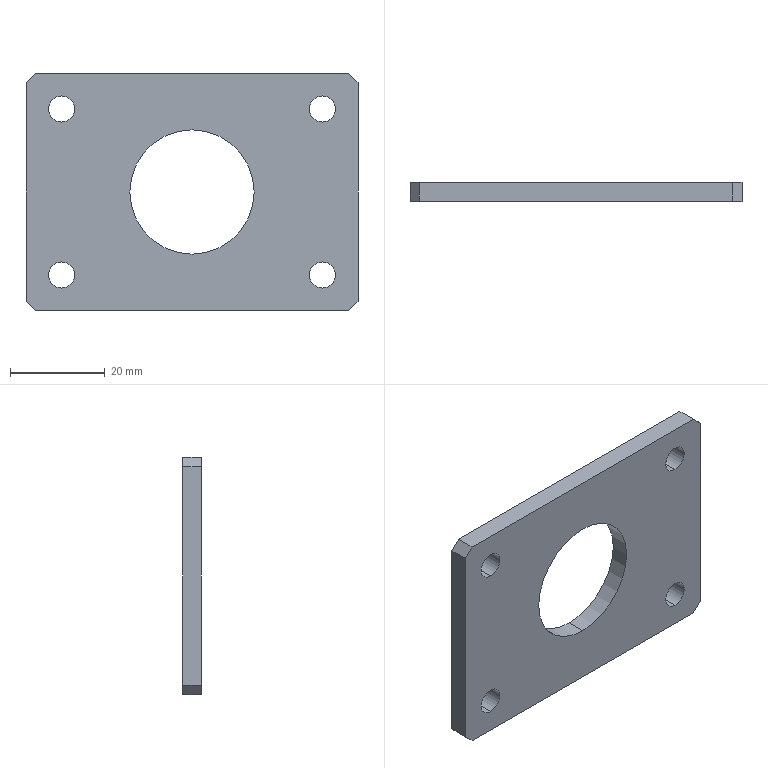Part | STEP file | BPSP-03-038Support Cylinder Fixing Plate_Default | 1 solid | 20 faces | box 70 x 4 x 50 mm | volume 11431 mm3 | cylinder 10 | plane 10 | commonest cylinder face diameters 5.5 x8 26.2 x2
STEP:
#1=CARTESIAN_POINT('',(0.,0.,0.));
#2=DIRECTION('',(0.,0.,1.));
#3=DIRECTION('',(1.,0.,0.));
#4=AXIS2_PLACEMENT_3D('',#1,#2,#3);
#5=CARTESIAN_POINT('',(27.5,-4.,-14.75));
#6=VERTEX_POINT('',#5);
#7=CARTESIAN_POINT('',(27.5,0.,-14.75));
#8=VERTEX_POINT('',#7);
#9=CARTESIAN_POINT('',(27.5,0.,-14.75));
#10=DIRECTION('',(0.,1.,0.));
#11=VECTOR('',#10,1.);
#12=LINE('',#9,#11);
#13=CARTESIAN_POINT('',(27.5,0.,-17.5));
#14=DIRECTION('',(0.,1.,0.));
#15=DIRECTION('',(0.,0.,1.));
#16=AXIS2_PLACEMENT_3D('',#13,#14,#15);
#17=CYLINDRICAL_SURFACE('',#16,2.75);
#18=CARTESIAN_POINT('',(6.283,0.));
#19=DIRECTION('',(0.,1.));
#20=VECTOR('',#19,1.);
#21=LINE('',#18,#20);
#22=(GEOMETRIC_REPRESENTATION_CONTEXT(2)PARAMETRIC_REPRESENTATION_CONTEXT()REPRESENTATION_CONTEXT('',''));
#23=DEFINITIONAL_REPRESENTATION('',(#21),#22);
#24=PCURVE('',#17,#23);
#25=CARTESIAN_POINT('',(27.5,0.,-17.5));
#26=DIRECTION('',(0.,1.,0.));
#27=DIRECTION('',(0.,0.,1.));
#28=AXIS2_PLACEMENT_3D('',#25,#26,#27);
#29=CYLINDRICAL_SURFACE('',#28,2.75);
#30=CARTESIAN_POINT('',(0.,0.));
#31=DIRECTION('',(0.,1.));
#32=VECTOR('',#31,1.);
#33=LINE('',#30,#32);
#34=(GEOMETRIC_REPRESENTATION_CONTEXT(2)PARAMETRIC_REPRESENTATION_CONTEXT()REPRESENTATION_CONTEXT('',''));
#35=DEFINITIONAL_REPRESENTATION('',(#33),#34);
#36=PCURVE('',#29,#35);
#37=SURFACE_CURVE('',#12,(#24,#36),.PCURVE_S1.);
#38=EDGE_CURVE('',#6,#8,#37,.T.);
#39=ORIENTED_EDGE('',*,*,#38,.T.);
#40=CARTESIAN_POINT('',(27.5,0.,-20.25));
#41=VERTEX_POINT('',#40);
#42=CARTESIAN_POINT('',(27.5,0.,-17.5));
#43=DIRECTION('',(0.,1.,0.));
#44=DIRECTION('',(0.,0.,1.));
#45=AXIS2_PLACEMENT_3D('',#42,#43,#44);
#46=CIRCLE('',#45,2.75);
#47=CARTESIAN_POINT('',(0.,0.));
#48=DIRECTION('',(1.,0.));
#49=VECTOR('',#48,1.);
#50=LINE('',#47,#49);
#51=(GEOMETRIC_REPRESENTATION_CONTEXT(2)PARAMETRIC_REPRESENTATION_CONTEXT()REPRESENTATION_CONTEXT('',''));
#52=DEFINITIONAL_REPRESENTATION('',(#50),#51);
#53=PCURVE('',#17,#52);
#54=CARTESIAN_POINT('',(0.,0.,0.));
#55=DIRECTION('',(0.,1.,0.));
#56=DIRECTION('',(0.,0.,1.));
#57=AXIS2_PLACEMENT_3D('',#54,#55,#56);
#58=PLANE('',#57);
#59=CARTESIAN_POINT('',(-17.5,27.5));
#60=DIRECTION('',(1.,0.));
#61=AXIS2_PLACEMENT_2D('',#59,#60);
#62=CIRCLE('',#61,2.75);
#63=(GEOMETRIC_REPRESENTATION_CONTEXT(2)PARAMETRIC_REPRESENTATION_CONTEXT()REPRESENTATION_CONTEXT('',''));
#64=DEFINITIONAL_REPRESENTATION('',(#62),#63);
#65=PCURVE('',#58,#64);
#66=SURFACE_CURVE('',#46,(#53,#65),.PCURVE_S1.);
#67=EDGE_CURVE('',#41,#8,#66,.T.);
#68=ORIENTED_EDGE('',*,*,#67,.F.);
#69=CARTESIAN_POINT('',(27.5,-4.,-20.25));
#70=VERTEX_POINT('',#69);
#71=CARTESIAN_POINT('',(27.5,0.,-20.25));
#72=DIRECTION('',(0.,1.,0.));
#73=VECTOR('',#72,1.);
#74=LINE('',#71,#73);
#75=CARTESIAN_POINT('',(3.142,0.));
#76=DIRECTION('',(0.,1.));
#77=VECTOR('',#76,1.);
#78=LINE('',#75,#77);
#79=(GEOMETRIC_REPRESENTATION_CONTEXT(2)PARAMETRIC_REPRESENTATION_CONTEXT()REPRESENTATION_CONTEXT('',''));
#80=DEFINITIONAL_REPRESENTATION('',(#78),#79);
#81=PCURVE('',#17,#80);
#82=CARTESIAN_POINT('',(3.142,0.));
#83=DIRECTION('',(0.,1.));
#84=VECTOR('',#83,1.);
#85=LINE('',#82,#84);
#86=(GEOMETRIC_REPRESENTATION_CONTEXT(2)PARAMETRIC_REPRESENTATION_CONTEXT()REPRESENTATION_CONTEXT('',''));
#87=DEFINITIONAL_REPRESENTATION('',(#85),#86);
#88=PCURVE('',#29,#87);
#89=SURFACE_CURVE('',#74,(#81,#88),.PCURVE_S1.);
#90=EDGE_CURVE('',#70,#41,#89,.T.);
#91=ORIENTED_EDGE('',*,*,#90,.F.);
#92=CARTESIAN_POINT('',(27.5,-4.,-17.5));
#93=DIRECTION('',(0.,1.,0.));
#94=DIRECTION('',(0.,0.,1.));
#95=AXIS2_PLACEMENT_3D('',#92,#93,#94);
#96=CIRCLE('',#95,2.75);
#97=CARTESIAN_POINT('',(0.,-4.));
#98=DIRECTION('',(1.,0.));
#99=VECTOR('',#98,1.);
#100=LINE('',#97,#99);
#101=(GEOMETRIC_REPRESENTATION_CONTEXT(2)PARAMETRIC_REPRESENTATION_CONTEXT()REPRESENTATION_CONTEXT('',''));
#102=DEFINITIONAL_REPRESENTATION('',(#100),#101);
#103=PCURVE('',#17,#102);
#104=CARTESIAN_POINT('',(0.,-4.,0.));
#105=DIRECTION('',(0.,1.,0.));
#106=DIRECTION('',(0.,0.,1.));
#107=AXIS2_PLACEMENT_3D('',#104,#105,#106);
#108=PLANE('',#107);
#109=CARTESIAN_POINT('',(-17.5,27.5));
#110=DIRECTION('',(1.,0.));
#111=AXIS2_PLACEMENT_2D('',#109,#110);
#112=CIRCLE('',#111,2.75);
#113=(GEOMETRIC_REPRESENTATION_CONTEXT(2)PARAMETRIC_REPRESENTATION_CONTEXT()REPRESENTATION_CONTEXT('',''));
#114=DEFINITIONAL_REPRESENTATION('',(#112),#113);
#115=PCURVE('',#108,#114);
#116=SURFACE_CURVE('',#96,(#103,#115),.PCURVE_S1.);
#117=EDGE_CURVE('',#70,#6,#116,.T.);
#118=ORIENTED_EDGE('',*,*,#117,.T.);
#119=EDGE_LOOP('',(#39,#68,#91,#118));
#120=FACE_BOUND('',#119,.F.);
#121=ADVANCED_FACE('',(#120),#17,.F.);
#122=CARTESIAN_POINT('',(-27.5,-4.,-14.75));
#123=VERTEX_POINT('',#122);
#124=CARTESIAN_POINT('',(-27.5,0.,-14.75));
#125=VERTEX_POINT('',#124);
#126=CARTESIAN_POINT('',(-27.5,0.,-14.75));
#127=DIRECTION('',(0.,1.,0.));
#128=VECTOR('',#127,1.);
#129=LINE('',#126,#128);
#130=CARTESIAN_POINT('',(-27.5,0.,-17.5));
#131=DIRECTION('',(0.,1.,0.));
#132=DIRECTION('',(0.,0.,1.));
#133=AXIS2_PLACEMENT_3D('',#130,#131,#132);
#134=CYLINDRICAL_SURFACE('',#133,2.75);
#135=CARTESIAN_POINT('',(6.283,0.));
#136=DIRECTION('',(0.,1.));
#137=VECTOR('',#136,1.);
#138=LINE('',#135,#137);
#139=(GEOMETRIC_REPRESENTATION_CONTEXT(2)PARAMETRIC_REPRESENTATION_CONTEXT()REPRESENTATION_CONTEXT('',''));
#140=DEFINITIONAL_REPRESENTATION('',(#138),#139);
#141=PCURVE('',#134,#140);
#142=CARTESIAN_POINT('',(-27.5,0.,-17.5));
#143=DIRECTION('',(0.,1.,0.));
#144=DIRECTION('',(0.,0.,1.));
#145=AXIS2_PLACEMENT_3D('',#142,#143,#144);
#146=CYLINDRICAL_SURFACE('',#145,2.75);
#147=CARTESIAN_POINT('',(0.,0.));
#148=DIRECTION('',(0.,1.));
#149=VECTOR('',#148,1.);
#150=LINE('',#147,#149);
#151=(GEOMETRIC_REPRESENTATION_CONTEXT(2)PARAMETRIC_REPRESENTATION_CONTEXT()REPRESENTATION_CONTEXT('',''));
#152=DEFINITIONAL_REPRESENTATION('',(#150),#151);
#153=PCURVE('',#146,#152);
#154=SURFACE_CURVE('',#129,(#141,#153),.PCURVE_S1.);
#155=EDGE_CURVE('',#123,#125,#154,.T.);
#156=ORIENTED_EDGE('',*,*,#155,.T.);
#157=CARTESIAN_POINT('',(-27.5,0.,-20.25));
#158=VERTEX_POINT('',#157);
#159=CARTESIAN_POINT('',(-27.5,0.,-17.5));
#160=DIRECTION('',(0.,1.,0.));
#161=DIRECTION('',(0.,0.,1.));
#162=AXIS2_PLACEMENT_3D('',#159,#160,#161);
#163=CIRCLE('',#162,2.75);
#164=CARTESIAN_POINT('',(0.,0.));
#165=DIRECTION('',(1.,0.));
#166=VECTOR('',#165,1.);
#167=LINE('',#164,#166);
#168=(GEOMETRIC_REPRESENTATION_CONTEXT(2)PARAMETRIC_REPRESENTATION_CONTEXT()REPRESENTATION_CONTEXT('',''));
#169=DEFINITIONAL_REPRESENTATION('',(#167),#168);
#170=PCURVE('',#134,#169);
#171=CARTESIAN_POINT('',(-17.5,-27.5));
#172=DIRECTION('',(1.,0.));
#173=AXIS2_PLACEMENT_2D('',#171,#172);
#174=CIRCLE('',#173,2.75);
#175=(GEOMETRIC_REPRESENTATION_CONTEXT(2)PARAMETRIC_REPRESENTATION_CONTEXT()REPRESENTATION_CONTEXT('',''));
#176=DEFINITIONAL_REPRESENTATION('',(#174),#175);
#177=PCURVE('',#58,#176);
#178=SURFACE_CURVE('',#163,(#170,#177),.PCURVE_S1.);
#179=EDGE_CURVE('',#158,#125,#178,.T.);
#180=ORIENTED_EDGE('',*,*,#179,.F.);
#181=CARTESIAN_POINT('',(-27.5,-4.,-20.25));
#182=VERTEX_POINT('',#181);
#183=CARTESIAN_POINT('',(-27.5,0.,-20.25));
#184=DIRECTION('',(0.,1.,0.));
#185=VECTOR('',#184,1.);
#186=LINE('',#183,#185);
#187=CARTESIAN_POINT('',(3.142,0.));
#188=DIRECTION('',(0.,1.));
#189=VECTOR('',#188,1.);
#190=LINE('',#187,#189);
#191=(GEOMETRIC_REPRESENTATION_CONTEXT(2)PARAMETRIC_REPRESENTATION_CONTEXT()REPRESENTATION_CONTEXT('',''));
#192=DEFINITIONAL_REPRESENTATION('',(#190),#191);
#193=PCURVE('',#134,#192);
#194=CARTESIAN_POINT('',(3.142,0.));
#195=DIRECTION('',(0.,1.));
#196=VECTOR('',#195,1.);
#197=LINE('',#194,#196);
#198=(GEOMETRIC_REPRESENTATION_CONTEXT(2)PARAMETRIC_REPRESENTATION_CONTEXT()REPRESENTATION_CONTEXT('',''));
#199=DEFINITIONAL_REPRESENTATION('',(#197),#198);
#200=PCURVE('',#146,#199);
#201=SURFACE_CURVE('',#186,(#193,#200),.PCURVE_S1.);
#202=EDGE_CURVE('',#182,#158,#201,.T.);
#203=ORIENTED_EDGE('',*,*,#202,.F.);
#204=CARTESIAN_POINT('',(-27.5,-4.,-17.5));
#205=DIRECTION('',(0.,1.,0.));
#206=DIRECTION('',(0.,0.,1.));
#207=AXIS2_PLACEMENT_3D('',#204,#205,#206);
#208=CIRCLE('',#207,2.75);
#209=CARTESIAN_POINT('',(0.,-4.));
#210=DIRECTION('',(1.,0.));
#211=VECTOR('',#210,1.);
#212=LINE('',#209,#211);
#213=(GEOMETRIC_REPRESENTATION_CONTEXT(2)PARAMETRIC_REPRESENTATION_CONTEXT()REPRESENTATION_CONTEXT('',''));
#214=DEFINITIONAL_REPRESENTATION('',(#212),#213);
#215=PCURVE('',#134,#214);
#216=CARTESIAN_POINT('',(-17.5,-27.5));
#217=DIRECTION('',(1.,0.));
#218=AXIS2_PLACEMENT_2D('',#216,#217);
#219=CIRCLE('',#218,2.75);
#220=(GEOMETRIC_REPRESENTATION_CONTEXT(2)PARAMETRIC_REPRESENTATION_CONTEXT()REPRESENTATION_CONTEXT('',''));
#221=DEFINITIONAL_REPRESENTATION('',(#219),#220);
#222=PCURVE('',#108,#221);
#223=SURFACE_CURVE('',#208,(#215,#222),.PCURVE_S1.);
#224=EDGE_CURVE('',#182,#123,#223,.T.);
#225=ORIENTED_EDGE('',*,*,#224,.T.);
#226=EDGE_LOOP('',(#156,#180,#203,#225));
#227=FACE_BOUND('',#226,.F.);
#228=ADVANCED_FACE('',(#227),#134,.F.);
#229=CARTESIAN_POINT('',(-27.5,-4.,20.25));
#230=VERTEX_POINT('',#229);
#231=CARTESIAN_POINT('',(-27.5,0.,20.25));
#232=VERTEX_POINT('',#231);
#233=CARTESIAN_POINT('',(-27.5,0.,20.25));
#234=DIRECTION('',(0.,1.,0.));
#235=VECTOR('',#234,1.);
#236=LINE('',#233,#235);
#237=CARTESIAN_POINT('',(-27.5,0.,17.5));
#238=DIRECTION('',(0.,1.,0.));
#239=DIRECTION('',(0.,0.,1.));
#240=AXIS2_PLACEMENT_3D('',#237,#238,#239);
#241=CYLINDRICAL_SURFACE('',#240,2.75);
#242=CARTESIAN_POINT('',(6.283,0.));
#243=DIRECTION('',(0.,1.));
#244=VECTOR('',#243,1.);
#245=LINE('',#242,#244);
#246=(GEOMETRIC_REPRESENTATION_CONTEXT(2)PARAMETRIC_REPRESENTATION_CONTEXT()REPRESENTATION_CONTEXT('',''));
#247=DEFINITIONAL_REPRESENTATION('',(#245),#246);
#248=PCURVE('',#241,#247);
#249=CARTESIAN_POINT('',(-27.5,0.,17.5));
#250=DIRECTION('',(0.,1.,0.));
#251=DIRECTION('',(0.,0.,1.));
#252=AXIS2_PLACEMENT_3D('',#249,#250,#251);
#253=CYLINDRICAL_SURFACE('',#252,2.75);
#254=CARTESIAN_POINT('',(0.,0.));
#255=DIRECTION('',(0.,1.));
#256=VECTOR('',#255,1.);
#257=LINE('',#254,#256);
#258=(GEOMETRIC_REPRESENTATION_CONTEXT(2)PARAMETRIC_REPRESENTATION_CONTEXT()REPRESENTATION_CONTEXT('',''));
#259=DEFINITIONAL_REPRESENTATION('',(#257),#258);
#260=PCURVE('',#253,#259);
#261=SURFACE_CURVE('',#236,(#248,#260),.PCURVE_S1.);
#262=EDGE_CURVE('',#230,#232,#261,.T.);
#263=ORIENTED_EDGE('',*,*,#262,.T.);
#264=CARTESIAN_POINT('',(-27.5,0.,14.75));
#265=VERTEX_POINT('',#264);
#266=CARTESIAN_POINT('',(-27.5,0.,17.5));
#267=DIRECTION('',(0.,1.,0.));
#268=DIRECTION('',(0.,0.,1.));
#269=AXIS2_PLACEMENT_3D('',#266,#267,#268);
#270=CIRCLE('',#269,2.75);
#271=CARTESIAN_POINT('',(0.,0.));
#272=DIRECTION('',(1.,0.));
#273=VECTOR('',#272,1.);
#274=LINE('',#271,#273);
#275=(GEOMETRIC_REPRESENTATION_CONTEXT(2)PARAMETRIC_REPRESENTATION_CONTEXT()REPRESENTATION_CONTEXT('',''));
#276=DEFINITIONAL_REPRESENTATION('',(#274),#275);
#277=PCURVE('',#241,#276);
#278=CARTESIAN_POINT('',(17.5,-27.5));
#279=DIRECTION('',(1.,0.));
#280=AXIS2_PLACEMENT_2D('',#278,#279);
#281=CIRCLE('',#280,2.75);
#282=(GEOMETRIC_REPRESENTATION_CONTEXT(2)PARAMETRIC_REPRESENTATION_CONTEXT()REPRESENTATION_CONTEXT('',''));
#283=DEFINITIONAL_REPRESENTATION('',(#281),#282);
#284=PCURVE('',#58,#283);
#285=SURFACE_CURVE('',#270,(#277,#284),.PCURVE_S1.);
#286=EDGE_CURVE('',#265,#232,#285,.T.);
#287=ORIENTED_EDGE('',*,*,#286,.F.);
#288=CARTESIAN_POINT('',(-27.5,-4.,14.75));
#289=VERTEX_POINT('',#288);
#290=CARTESIAN_POINT('',(-27.5,0.,14.75));
#291=DIRECTION('',(0.,1.,0.));
#292=VECTOR('',#291,1.);
#293=LINE('',#290,#292);
#294=CARTESIAN_POINT('',(3.142,0.));
#295=DIRECTION('',(0.,1.));
#296=VECTOR('',#295,1.);
#297=LINE('',#294,#296);
#298=(GEOMETRIC_REPRESENTATION_CONTEXT(2)PARAMETRIC_REPRESENTATION_CONTEXT()REPRESENTATION_CONTEXT('',''));
#299=DEFINITIONAL_REPRESENTATION('',(#297),#298);
#300=PCURVE('',#241,#299);
#301=CARTESIAN_POINT('',(3.142,0.));
#302=DIRECTION('',(0.,1.));
#303=VECTOR('',#302,1.);
#304=LINE('',#301,#303);
#305=(GEOMETRIC_REPRESENTATION_CONTEXT(2)PARAMETRIC_REPRESENTATION_CONTEXT()REPRESENTATION_CONTEXT('',''));
#306=DEFINITIONAL_REPRESENTATION('',(#304),#305);
#307=PCURVE('',#253,#306);
#308=SURFACE_CURVE('',#293,(#300,#307),.PCURVE_S1.);
#309=EDGE_CURVE('',#289,#265,#308,.T.);
#310=ORIENTED_EDGE('',*,*,#309,.F.);
#311=CARTESIAN_POINT('',(-27.5,-4.,17.5));
#312=DIRECTION('',(0.,1.,0.));
#313=DIRECTION('',(0.,0.,1.));
#314=AXIS2_PLACEMENT_3D('',#311,#312,#313);
#315=CIRCLE('',#314,2.75);
#316=CARTESIAN_POINT('',(0.,-4.));
#317=DIRECTION('',(1.,0.));
#318=VECTOR('',#317,1.);
#319=LINE('',#316,#318);
#320=(GEOMETRIC_REPRESENTATION_CONTEXT(2)PARAMETRIC_REPRESENTATION_CONTEXT()REPRESENTATION_CONTEXT('',''));
#321=DEFINITIONAL_REPRESENTATION('',(#319),#320);
#322=PCURVE('',#241,#321);
#323=CARTESIAN_POINT('',(17.5,-27.5));
#324=DIRECTION('',(1.,0.));
#325=AXIS2_PLACEMENT_2D('',#323,#324);
#326=CIRCLE('',#325,2.75);
#327=(GEOMETRIC_REPRESENTATION_CONTEXT(2)PARAMETRIC_REPRESENTATION_CONTEXT()REPRESENTATION_CONTEXT('',''));
#328=DEFINITIONAL_REPRESENTATION('',(#326),#327);
#329=PCURVE('',#108,#328);
#330=SURFACE_CURVE('',#315,(#322,#329),.PCURVE_S1.);
#331=EDGE_CURVE('',#289,#230,#330,.T.);
#332=ORIENTED_EDGE('',*,*,#331,.T.);
#333=EDGE_LOOP('',(#263,#287,#310,#332));
#334=FACE_BOUND('',#333,.F.);
#335=ADVANCED_FACE('',(#334),#241,.F.);
#336=CARTESIAN_POINT('',(27.5,-4.,20.25));
#337=VERTEX_POINT('',#336);
#338=CARTESIAN_POINT('',(27.5,0.,20.25));
#339=VERTEX_POINT('',#338);
#340=CARTESIAN_POINT('',(27.5,0.,20.25));
#341=DIRECTION('',(0.,1.,0.));
#342=VECTOR('',#341,1.);
#343=LINE('',#340,#342);
#344=CARTESIAN_POINT('',(27.5,0.,17.5));
#345=DIRECTION('',(0.,1.,0.));
#346=DIRECTION('',(0.,0.,1.));
#347=AXIS2_PLACEMENT_3D('',#344,#345,#346);
#348=CYLINDRICAL_SURFACE('',#347,2.75);
#349=CARTESIAN_POINT('',(6.283,0.));
#350=DIRECTION('',(0.,1.));
#351=VECTOR('',#350,1.);
#352=LINE('',#349,#351);
#353=(GEOMETRIC_REPRESENTATION_CONTEXT(2)PARAMETRIC_REPRESENTATION_CONTEXT()REPRESENTATION_CONTEXT('',''));
#354=DEFINITIONAL_REPRESENTATION('',(#352),#353);
#355=PCURVE('',#348,#354);
#356=CARTESIAN_POINT('',(27.5,0.,17.5));
#357=DIRECTION('',(0.,1.,0.));
#358=DIRECTION('',(0.,0.,1.));
#359=AXIS2_PLACEMENT_3D('',#356,#357,#358);
#360=CYLINDRICAL_SURFACE('',#359,2.75);
#361=CARTESIAN_POINT('',(0.,0.));
#362=DIRECTION('',(0.,1.));
#363=VECTOR('',#362,1.);
#364=LINE('',#361,#363);
#365=(GEOMETRIC_REPRESENTATION_CONTEXT(2)PARAMETRIC_REPRESENTATION_CONTEXT()REPRESENTATION_CONTEXT('',''));
#366=DEFINITIONAL_REPRESENTATION('',(#364),#365);
#367=PCURVE('',#360,#366);
#368=SURFACE_CURVE('',#343,(#355,#367),.PCURVE_S1.);
#369=EDGE_CURVE('',#337,#339,#368,.T.);
#370=ORIENTED_EDGE('',*,*,#369,.T.);
#371=CARTESIAN_POINT('',(27.5,0.,14.75));
#372=VERTEX_POINT('',#371);
#373=CARTESIAN_POINT('',(27.5,0.,17.5));
#374=DIRECTION('',(0.,1.,0.));
#375=DIRECTION('',(0.,0.,1.));
#376=AXIS2_PLACEMENT_3D('',#373,#374,#375);
#377=CIRCLE('',#376,2.75);
#378=CARTESIAN_POINT('',(0.,0.));
#379=DIRECTION('',(1.,0.));
#380=VECTOR('',#379,1.);
#381=LINE('',#378,#380);
#382=(GEOMETRIC_REPRESENTATION_CONTEXT(2)PARAMETRIC_REPRESENTATION_CONTEXT()REPRESENTATION_CONTEXT('',''));
#383=DEFINITIONAL_REPRESENTATION('',(#381),#382);
#384=PCURVE('',#348,#383);
#385=CARTESIAN_POINT('',(17.5,27.5));
#386=DIRECTION('',(1.,0.));
#387=AXIS2_PLACEMENT_2D('',#385,#386);
#388=CIRCLE('',#387,2.75);
#389=(GEOMETRIC_REPRESENTATION_CONTEXT(2)PARAMETRIC_REPRESENTATION_CONTEXT()REPRESENTATION_CONTEXT('',''));
#390=DEFINITIONAL_REPRESENTATION('',(#388),#389);
#391=PCURVE('',#58,#390);
#392=SURFACE_CURVE('',#377,(#384,#391),.PCURVE_S1.);
#393=EDGE_CURVE('',#372,#339,#392,.T.);
#394=ORIENTED_EDGE('',*,*,#393,.F.);
#395=CARTESIAN_POINT('',(27.5,-4.,14.75));
#396=VERTEX_POINT('',#395);
#397=CARTESIAN_POINT('',(27.5,0.,14.75));
#398=DIRECTION('',(0.,1.,0.));
#399=VECTOR('',#398,1.);
#400=LINE('',#397,#399);
#401=CARTESIAN_POINT('',(3.142,0.));
#402=DIRECTION('',(0.,1.));
#403=VECTOR('',#402,1.);
#404=LINE('',#401,#403);
#405=(GEOMETRIC_REPRESENTATION_CONTEXT(2)PARAMETRIC_REPRESENTATION_CONTEXT()REPRESENTATION_CONTEXT('',''));
#406=DEFINITIONAL_REPRESENTATION('',(#404),#405);
#407=PCURVE('',#348,#406);
#408=CARTESIAN_POINT('',(3.142,0.));
#409=DIRECTION('',(0.,1.));
#410=VECTOR('',#409,1.);
#411=LINE('',#408,#410);
#412=(GEOMETRIC_REPRESENTATION_CONTEXT(2)PARAMETRIC_REPRESENTATION_CONTEXT()REPRESENTATION_CONTEXT('',''));
#413=DEFINITIONAL_REPRESENTATION('',(#411),#412);
#414=PCURVE('',#360,#413);
#415=SURFACE_CURVE('',#400,(#407,#414),.PCURVE_S1.);
#416=EDGE_CURVE('',#396,#372,#415,.T.);
#417=ORIENTED_EDGE('',*,*,#416,.F.);
#418=CARTESIAN_POINT('',(27.5,-4.,17.5));
#419=DIRECTION('',(0.,1.,0.));
#420=DIRECTION('',(0.,0.,1.));
#421=AXIS2_PLACEMENT_3D('',#418,#419,#420);
#422=CIRCLE('',#421,2.75);
#423=CARTESIAN_POINT('',(0.,-4.));
#424=DIRECTION('',(1.,0.));
#425=VECTOR('',#424,1.);
#426=LINE('',#423,#425);
#427=(GEOMETRIC_REPRESENTATION_CONTEXT(2)PARAMETRIC_REPRESENTATION_CONTEXT()REPRESENTATION_CONTEXT('',''));
#428=DEFINITIONAL_REPRESENTATION('',(#426),#427);
#429=PCURVE('',#348,#428);
#430=CARTESIAN_POINT('',(17.5,27.5));
#431=DIRECTION('',(1.,0.));
#432=AXIS2_PLACEMENT_2D('',#430,#431);
#433=CIRCLE('',#432,2.75);
#434=(GEOMETRIC_REPRESENTATION_CONTEXT(2)PARAMETRIC_REPRESENTATION_CONTEXT()REPRESENTATION_CONTEXT('',''));
#435=DEFINITIONAL_REPRESENTATION('',(#433),#434);
#436=PCURVE('',#108,#435);
#437=SURFACE_CURVE('',#422,(#429,#436),.PCURVE_S1.);
#438=EDGE_CURVE('',#396,#337,#437,.T.);
#439=ORIENTED_EDGE('',*,*,#438,.T.);
#440=EDGE_LOOP('',(#370,#394,#417,#439));
#441=FACE_BOUND('',#440,.F.);
#442=ADVANCED_FACE('',(#441),#348,.F.);
#443=CARTESIAN_POINT('',(0.,-4.,13.1));
#444=VERTEX_POINT('',#443);
#445=CARTESIAN_POINT('',(0.,0.,13.1));
#446=VERTEX_POINT('',#445);
#447=CARTESIAN_POINT('',(0.,-4.,13.1));
#448=DIRECTION('',(0.,1.,0.));
#449=VECTOR('',#448,1.);
#450=LINE('',#447,#449);
#451=CARTESIAN_POINT('',(0.,-4.,0.));
#452=DIRECTION('',(0.,1.,0.));
#453=DIRECTION('',(0.,0.,1.));
#454=AXIS2_PLACEMENT_3D('',#451,#452,#453);
#455=CYLINDRICAL_SURFACE('',#454,13.1);
#456=CARTESIAN_POINT('',(6.283,0.));
#457=DIRECTION('',(0.,1.));
#458=VECTOR('',#457,1.);
#459=LINE('',#456,#458);
#460=(GEOMETRIC_REPRESENTATION_CONTEXT(2)PARAMETRIC_REPRESENTATION_CONTEXT()REPRESENTATION_CONTEXT('',''));
#461=DEFINITIONAL_REPRESENTATION('',(#459),#460);
#462=PCURVE('',#455,#461);
#463=CARTESIAN_POINT('',(0.,-4.,0.));
#464=DIRECTION('',(0.,1.,0.));
#465=DIRECTION('',(0.,0.,1.));
#466=AXIS2_PLACEMENT_3D('',#463,#464,#465);
#467=CYLINDRICAL_SURFACE('',#466,13.1);
#468=CARTESIAN_POINT('',(0.,0.));
#469=DIRECTION('',(0.,1.));
#470=VECTOR('',#469,1.);
#471=LINE('',#468,#470);
#472=(GEOMETRIC_REPRESENTATION_CONTEXT(2)PARAMETRIC_REPRESENTATION_CONTEXT()REPRESENTATION_CONTEXT('',''));
#473=DEFINITIONAL_REPRESENTATION('',(#471),#472);
#474=PCURVE('',#467,#473);
#475=SURFACE_CURVE('',#450,(#462,#474),.PCURVE_S1.);
#476=EDGE_CURVE('',#444,#446,#475,.T.);
#477=ORIENTED_EDGE('',*,*,#476,.T.);
#478=CARTESIAN_POINT('',(0.,0.,-13.1));
#479=VERTEX_POINT('',#478);
#480=CARTESIAN_POINT('',(0.,0.,0.));
#481=DIRECTION('',(0.,1.,0.));
#482=DIRECTION('',(0.,0.,1.));
#483=AXIS2_PLACEMENT_3D('',#480,#481,#482);
#484=CIRCLE('',#483,13.1);
#485=CARTESIAN_POINT('',(0.,4.));
#486=DIRECTION('',(1.,0.));
#487=VECTOR('',#486,1.);
#488=LINE('',#485,#487);
#489=(GEOMETRIC_REPRESENTATION_CONTEXT(2)PARAMETRIC_REPRESENTATION_CONTEXT()REPRESENTATION_CONTEXT('',''));
#490=DEFINITIONAL_REPRESENTATION('',(#488),#489);
#491=PCURVE('',#455,#490);
#492=CARTESIAN_POINT('',(0.,0.));
#493=DIRECTION('',(1.,0.));
#494=AXIS2_PLACEMENT_2D('',#492,#493);
#495=CIRCLE('',#494,13.1);
#496=(GEOMETRIC_REPRESENTATION_CONTEXT(2)PARAMETRIC_REPRESENTATION_CONTEXT()REPRESENTATION_CONTEXT('',''));
#497=DEFINITIONAL_REPRESENTATION('',(#495),#496);
#498=PCURVE('',#58,#497);
#499=SURFACE_CURVE('',#484,(#491,#498),.PCURVE_S1.);
#500=EDGE_CURVE('',#479,#446,#499,.T.);
#501=ORIENTED_EDGE('',*,*,#500,.F.);
#502=CARTESIAN_POINT('',(0.,-4.,-13.1));
#503=VERTEX_POINT('',#502);
#504=CARTESIAN_POINT('',(0.,-4.,-13.1));
#505=DIRECTION('',(0.,1.,0.));
#506=VECTOR('',#505,1.);
#507=LINE('',#504,#506);
#508=CARTESIAN_POINT('',(3.142,0.));
#509=DIRECTION('',(0.,1.));
#510=VECTOR('',#509,1.);
#511=LINE('',#508,#510);
#512=(GEOMETRIC_REPRESENTATION_CONTEXT(2)PARAMETRIC_REPRESENTATION_CONTEXT()REPRESENTATION_CONTEXT('',''));
#513=DEFINITIONAL_REPRESENTATION('',(#511),#512);
#514=PCURVE('',#455,#513);
#515=CARTESIAN_POINT('',(3.142,0.));
#516=DIRECTION('',(0.,1.));
#517=VECTOR('',#516,1.);
#518=LINE('',#515,#517);
#519=(GEOMETRIC_REPRESENTATION_CONTEXT(2)PARAMETRIC_REPRESENTATION_CONTEXT()REPRESENTATION_CONTEXT('',''));
#520=DEFINITIONAL_REPRESENTATION('',(#518),#519);
#521=PCURVE('',#467,#520);
#522=SURFACE_CURVE('',#507,(#514,#521),.PCURVE_S1.);
#523=EDGE_CURVE('',#503,#479,#522,.T.);
#524=ORIENTED_EDGE('',*,*,#523,.F.);
#525=CARTESIAN_POINT('',(0.,-4.,0.));
#526=DIRECTION('',(0.,1.,0.));
#527=DIRECTION('',(0.,0.,1.));
#528=AXIS2_PLACEMENT_3D('',#525,#526,#527);
#529=CIRCLE('',#528,13.1);
#530=CARTESIAN_POINT('',(0.,0.));
#531=DIRECTION('',(1.,0.));
#532=VECTOR('',#531,1.);
#533=LINE('',#530,#532);
#534=(GEOMETRIC_REPRESENTATION_CONTEXT(2)PARAMETRIC_REPRESENTATION_CONTEXT()REPRESENTATION_CONTEXT('',''));
#535=DEFINITIONAL_REPRESENTATION('',(#533),#534);
#536=PCURVE('',#455,#535);
#537=CARTESIAN_POINT('',(0.,0.));
#538=DIRECTION('',(1.,0.));
#539=AXIS2_PLACEMENT_2D('',#537,#538);
#540=CIRCLE('',#539,13.1);
#541=(GEOMETRIC_REPRESENTATION_CONTEXT(2)PARAMETRIC_REPRESENTATION_CONTEXT()REPRESENTATION_CONTEXT('',''));
#542=DEFINITIONAL_REPRESENTATION('',(#540),#541);
#543=PCURVE('',#108,#542);
#544=SURFACE_CURVE('',#529,(#536,#543),.PCURVE_S1.);
#545=EDGE_CURVE('',#503,#444,#544,.T.);
#546=ORIENTED_EDGE('',*,*,#545,.T.);
#547=EDGE_LOOP('',(#477,#501,#524,#546));
#548=FACE_BOUND('',#547,.F.);
#549=ADVANCED_FACE('',(#548),#455,.F.);
#550=CARTESIAN_POINT('',(35.,-4.,23.));
#551=VERTEX_POINT('',#550);
#552=CARTESIAN_POINT('',(35.,-4.,-23.));
#553=VERTEX_POINT('',#552);
#554=CARTESIAN_POINT('',(35.,-4.,-25.));
#555=DIRECTION('',(0.,0.,-1.));
#556=VECTOR('',#555,1.);
#557=LINE('',#554,#556);
#558=CARTESIAN_POINT('',(35.,-4.,-25.));
#559=DIRECTION('',(1.,0.,0.));
#560=DIRECTION('',(0.,0.,-1.));
#561=AXIS2_PLACEMENT_3D('',#558,#559,#560);
#562=PLANE('',#561);
#563=CARTESIAN_POINT('',(0.,0.));
#564=DIRECTION('',(1.,0.));
#565=VECTOR('',#564,1.);
#566=LINE('',#563,#565);
#567=(GEOMETRIC_REPRESENTATION_CONTEXT(2)PARAMETRIC_REPRESENTATION_CONTEXT()REPRESENTATION_CONTEXT('',''));
#568=DEFINITIONAL_REPRESENTATION('',(#566),#567);
#569=PCURVE('',#562,#568);
#570=CARTESIAN_POINT('',(-25.,35.));
#571=DIRECTION('',(-1.,0.));
#572=VECTOR('',#571,1.);
#573=LINE('',#570,#572);
#574=(GEOMETRIC_REPRESENTATION_CONTEXT(2)PARAMETRIC_REPRESENTATION_CONTEXT()REPRESENTATION_CONTEXT('',''));
#575=DEFINITIONAL_REPRESENTATION('',(#573),#574);
#576=PCURVE('',#108,#575);
#577=SURFACE_CURVE('',#557,(#569,#576),.PCURVE_S1.);
#578=EDGE_CURVE('',#551,#553,#577,.T.);
#579=ORIENTED_EDGE('',*,*,#578,.T.);
#580=CARTESIAN_POINT('',(35.,0.,-23.));
#581=VERTEX_POINT('',#580);
#582=CARTESIAN_POINT('',(35.,-4.,-23.));
#583=DIRECTION('',(0.,1.,0.));
#584=VECTOR('',#583,1.);
#585=LINE('',#582,#584);
#586=CARTESIAN_POINT('',(-2.,0.));
#587=DIRECTION('',(0.,1.));
#588=VECTOR('',#587,1.);
#589=LINE('',#586,#588);
#590=(GEOMETRIC_REPRESENTATION_CONTEXT(2)PARAMETRIC_REPRESENTATION_CONTEXT()REPRESENTATION_CONTEXT('',''));
#591=DEFINITIONAL_REPRESENTATION('',(#589),#590);
#592=PCURVE('',#562,#591);
#593=CARTESIAN_POINT('',(35.,-4.,-23.));
#594=DIRECTION('',(-0.7071,0.,0.7071));
#595=DIRECTION('',(0.,1.,0.));
#596=AXIS2_PLACEMENT_3D('',#593,#594,#595);
#597=PLANE('',#596);
#598=CARTESIAN_POINT('',(0.,0.));
#599=DIRECTION('',(1.,0.));
#600=VECTOR('',#599,1.);
#601=LINE('',#598,#600);
#602=(GEOMETRIC_REPRESENTATION_CONTEXT(2)PARAMETRIC_REPRESENTATION_CONTEXT()REPRESENTATION_CONTEXT('',''));
#603=DEFINITIONAL_REPRESENTATION('',(#601),#602);
#604=PCURVE('',#597,#603);
#605=SURFACE_CURVE('',#585,(#592,#604),.PCURVE_S1.);
#606=EDGE_CURVE('',#553,#581,#605,.T.);
#607=ORIENTED_EDGE('',*,*,#606,.T.);
#608=CARTESIAN_POINT('',(35.,0.,23.));
#609=VERTEX_POINT('',#608);
#610=CARTESIAN_POINT('',(35.,0.,-25.));
#611=DIRECTION('',(0.,0.,-1.));
#612=VECTOR('',#611,1.);
#613=LINE('',#610,#612);
#614=CARTESIAN_POINT('',(0.,4.));
#615=DIRECTION('',(1.,0.));
#616=VECTOR('',#615,1.);
#617=LINE('',#614,#616);
#618=(GEOMETRIC_REPRESENTATION_CONTEXT(2)PARAMETRIC_REPRESENTATION_CONTEXT()REPRESENTATION_CONTEXT('',''));
#619=DEFINITIONAL_REPRESENTATION('',(#617),#618);
#620=PCURVE('',#562,#619);
#621=CARTESIAN_POINT('',(-25.,35.));
#622=DIRECTION('',(-1.,0.));
#623=VECTOR('',#622,1.);
#624=LINE('',#621,#623);
#625=(GEOMETRIC_REPRESENTATION_CONTEXT(2)PARAMETRIC_REPRESENTATION_CONTEXT()REPRESENTATION_CONTEXT('',''));
#626=DEFINITIONAL_REPRESENTATION('',(#624),#625);
#627=PCURVE('',#58,#626);
#628=SURFACE_CURVE('',#613,(#620,#627),.PCURVE_S1.);
#629=EDGE_CURVE('',#609,#581,#628,.T.);
#630=ORIENTED_EDGE('',*,*,#629,.F.);
#631=CARTESIAN_POINT('',(35.,-4.,23.));
#632=DIRECTION('',(0.,-1.,0.));
#633=VECTOR('',#632,1.);
#634=LINE('',#631,#633);
#635=CARTESIAN_POINT('',(-48.,0.));
#636=DIRECTION('',(0.,-1.));
#637=VECTOR('',#636,1.);
#638=LINE('',#635,#637);
#639=(GEOMETRIC_REPRESENTATION_CONTEXT(2)PARAMETRIC_REPRESENTATION_CONTEXT()REPRESENTATION_CONTEXT('',''));
#640=DEFINITIONAL_REPRESENTATION('',(#638),#639);
#641=PCURVE('',#562,#640);
#642=CARTESIAN_POINT('',(33.,-4.,25.));
#643=DIRECTION('',(-0.7071,0.,-0.7071));
#644=DIRECTION('',(0.,1.,0.));
#645=AXIS2_PLACEMENT_3D('',#642,#643,#644);
#646=PLANE('',#645);
#647=CARTESIAN_POINT('',(0.,2.828));
#648=DIRECTION('',(-1.,0.));
#649=VECTOR('',#648,1.);
#650=LINE('',#647,#649);
#651=(GEOMETRIC_REPRESENTATION_CONTEXT(2)PARAMETRIC_REPRESENTATION_CONTEXT()REPRESENTATION_CONTEXT('',''));
#652=DEFINITIONAL_REPRESENTATION('',(#650),#651);
#653=PCURVE('',#646,#652);
#654=SURFACE_CURVE('',#634,(#641,#653),.PCURVE_S1.);
#655=EDGE_CURVE('',#609,#551,#654,.T.);
#656=ORIENTED_EDGE('',*,*,#655,.T.);
#657=EDGE_LOOP('',(#579,#607,#630,#656));
#658=FACE_BOUND('',#657,.T.);
#659=ADVANCED_FACE('',(#658),#562,.T.);
#660=CARTESIAN_POINT('',(-33.,-4.,25.));
#661=VERTEX_POINT('',#660);
#662=CARTESIAN_POINT('',(33.,-4.,25.));
#663=VERTEX_POINT('',#662);
#664=CARTESIAN_POINT('',(-35.,-4.,25.));
#665=DIRECTION('',(1.,0.,0.));
#666=VECTOR('',#665,1.);
#667=LINE('',#664,#666);
#668=CARTESIAN_POINT('',(-35.,-4.,25.));
#669=DIRECTION('',(0.,0.,1.));
#670=DIRECTION('',(1.,0.,0.));
#671=AXIS2_PLACEMENT_3D('',#668,#669,#670);
#672=PLANE('',#671);
#673=CARTESIAN_POINT('',(0.,0.));
#674=DIRECTION('',(1.,0.));
#675=VECTOR('',#674,1.);
#676=LINE('',#673,#675);
#677=(GEOMETRIC_REPRESENTATION_CONTEXT(2)PARAMETRIC_REPRESENTATION_CONTEXT()REPRESENTATION_CONTEXT('',''));
#678=DEFINITIONAL_REPRESENTATION('',(#676),#677);
#679=PCURVE('',#672,#678);
#680=CARTESIAN_POINT('',(25.,-35.));
#681=DIRECTION('',(0.,1.));
#682=VECTOR('',#681,1.);
#683=LINE('',#680,#682);
#684=(GEOMETRIC_REPRESENTATION_CONTEXT(2)PARAMETRIC_REPRESENTATION_CONTEXT()REPRESENTATION_CONTEXT('',''));
#685=DEFINITIONAL_REPRESENTATION('',(#683),#684);
#686=PCURVE('',#108,#685);
#687=SURFACE_CURVE('',#667,(#679,#686),.PCURVE_S1.);
#688=EDGE_CURVE('',#661,#663,#687,.T.);
#689=ORIENTED_EDGE('',*,*,#688,.T.);
#690=CARTESIAN_POINT('',(33.,0.,25.));
#691=VERTEX_POINT('',#690);
#692=CARTESIAN_POINT('',(33.,-4.,25.));
#693=DIRECTION('',(0.,1.,0.));
#694=VECTOR('',#693,1.);
#695=LINE('',#692,#694);
#696=CARTESIAN_POINT('',(68.,0.));
#697=DIRECTION('',(0.,1.));
#698=VECTOR('',#697,1.);
#699=LINE('',#696,#698);
#700=(GEOMETRIC_REPRESENTATION_CONTEXT(2)PARAMETRIC_REPRESENTATION_CONTEXT()REPRESENTATION_CONTEXT('',''));
#701=DEFINITIONAL_REPRESENTATION('',(#699),#700);
#702=PCURVE('',#672,#701);
#703=CARTESIAN_POINT('',(0.,0.));
#704=DIRECTION('',(1.,0.));
#705=VECTOR('',#704,1.);
#706=LINE('',#703,#705);
#707=(GEOMETRIC_REPRESENTATION_CONTEXT(2)PARAMETRIC_REPRESENTATION_CONTEXT()REPRESENTATION_CONTEXT('',''));
#708=DEFINITIONAL_REPRESENTATION('',(#706),#707);
#709=PCURVE('',#646,#708);
#710=SURFACE_CURVE('',#695,(#702,#709),.PCURVE_S1.);
#711=EDGE_CURVE('',#663,#691,#710,.T.);
#712=ORIENTED_EDGE('',*,*,#711,.T.);
#713=CARTESIAN_POINT('',(-33.,0.,25.));
#714=VERTEX_POINT('',#713);
#715=CARTESIAN_POINT('',(-35.,0.,25.));
#716=DIRECTION('',(1.,0.,0.));
#717=VECTOR('',#716,1.);
#718=LINE('',#715,#717);
#719=CARTESIAN_POINT('',(0.,4.));
#720=DIRECTION('',(1.,0.));
#721=VECTOR('',#720,1.);
#722=LINE('',#719,#721);
#723=(GEOMETRIC_REPRESENTATION_CONTEXT(2)PARAMETRIC_REPRESENTATION_CONTEXT()REPRESENTATION_CONTEXT('',''));
#724=DEFINITIONAL_REPRESENTATION('',(#722),#723);
#725=PCURVE('',#672,#724);
#726=CARTESIAN_POINT('',(25.,-35.));
#727=DIRECTION('',(0.,1.));
#728=VECTOR('',#727,1.);
#729=LINE('',#726,#728);
#730=(GEOMETRIC_REPRESENTATION_CONTEXT(2)PARAMETRIC_REPRESENTATION_CONTEXT()REPRESENTATION_CONTEXT('',''));
#731=DEFINITIONAL_REPRESENTATION('',(#729),#730);
#732=PCURVE('',#58,#731);
#733=SURFACE_CURVE('',#718,(#725,#732),.PCURVE_S1.);
#734=EDGE_CURVE('',#714,#691,#733,.T.);
#735=ORIENTED_EDGE('',*,*,#734,.F.);
#736=CARTESIAN_POINT('',(-33.,-4.,25.));
#737=DIRECTION('',(0.,-1.,0.));
#738=VECTOR('',#737,1.);
#739=LINE('',#736,#738);
#740=CARTESIAN_POINT('',(2.,0.));
#741=DIRECTION('',(0.,-1.));
#742=VECTOR('',#741,1.);
#743=LINE('',#740,#742);
#744=(GEOMETRIC_REPRESENTATION_CONTEXT(2)PARAMETRIC_REPRESENTATION_CONTEXT()REPRESENTATION_CONTEXT('',''));
#745=DEFINITIONAL_REPRESENTATION('',(#743),#744);
#746=PCURVE('',#672,#745);
#747=CARTESIAN_POINT('',(-35.,-4.,23.));
#748=DIRECTION('',(0.7071,0.,-0.7071));
#749=DIRECTION('',(0.,1.,0.));
#750=AXIS2_PLACEMENT_3D('',#747,#748,#749);
#751=PLANE('',#750);
#752=CARTESIAN_POINT('',(0.,2.828));
#753=DIRECTION('',(-1.,0.));
#754=VECTOR('',#753,1.);
#755=LINE('',#752,#754);
#756=(GEOMETRIC_REPRESENTATION_CONTEXT(2)PARAMETRIC_REPRESENTATION_CONTEXT()REPRESENTATION_CONTEXT('',''));
#757=DEFINITIONAL_REPRESENTATION('',(#755),#756);
#758=PCURVE('',#751,#757);
#759=SURFACE_CURVE('',#739,(#746,#758),.PCURVE_S1.);
#760=EDGE_CURVE('',#714,#661,#759,.T.);
#761=ORIENTED_EDGE('',*,*,#760,.T.);
#762=EDGE_LOOP('',(#689,#712,#735,#761));
#763=FACE_BOUND('',#762,.T.);
#764=ADVANCED_FACE('',(#763),#672,.T.);
#765=CARTESIAN_POINT('',(-35.,-4.,-23.));
#766=VERTEX_POINT('',#765);
#767=CARTESIAN_POINT('',(-35.,-4.,23.));
#768=VERTEX_POINT('',#767);
#769=CARTESIAN_POINT('',(-35.,-4.,-25.));
#770=DIRECTION('',(0.,0.,1.));
#771=VECTOR('',#770,1.);
#772=LINE('',#769,#771);
#773=CARTESIAN_POINT('',(-35.,-4.,-25.));
#774=DIRECTION('',(-1.,0.,0.));
#775=DIRECTION('',(0.,0.,1.));
#776=AXIS2_PLACEMENT_3D('',#773,#774,#775);
#777=PLANE('',#776);
#778=CARTESIAN_POINT('',(0.,0.));
#779=DIRECTION('',(1.,0.));
#780=VECTOR('',#779,1.);
#781=LINE('',#778,#780);
#782=(GEOMETRIC_REPRESENTATION_CONTEXT(2)PARAMETRIC_REPRESENTATION_CONTEXT()REPRESENTATION_CONTEXT('',''));
#783=DEFINITIONAL_REPRESENTATION('',(#781),#782);
#784=PCURVE('',#777,#783);
#785=CARTESIAN_POINT('',(-25.,-35.));
#786=DIRECTION('',(1.,0.));
#787=VECTOR('',#786,1.);
#788=LINE('',#785,#787);
#789=(GEOMETRIC_REPRESENTATION_CONTEXT(2)PARAMETRIC_REPRESENTATION_CONTEXT()REPRESENTATION_CONTEXT('',''));
#790=DEFINITIONAL_REPRESENTATION('',(#788),#789);
#791=PCURVE('',#108,#790);
#792=SURFACE_CURVE('',#772,(#784,#791),.PCURVE_S1.);
#793=EDGE_CURVE('',#766,#768,#792,.T.);
#794=ORIENTED_EDGE('',*,*,#793,.T.);
#795=CARTESIAN_POINT('',(-35.,0.,23.));
#796=VERTEX_POINT('',#795);
#797=CARTESIAN_POINT('',(-35.,-4.,23.));
#798=DIRECTION('',(0.,1.,0.));
#799=VECTOR('',#798,1.);
#800=LINE('',#797,#799);
#801=CARTESIAN_POINT('',(48.,0.));
#802=DIRECTION('',(0.,1.));
#803=VECTOR('',#802,1.);
#804=LINE('',#801,#803);
#805=(GEOMETRIC_REPRESENTATION_CONTEXT(2)PARAMETRIC_REPRESENTATION_CONTEXT()REPRESENTATION_CONTEXT('',''));
#806=DEFINITIONAL_REPRESENTATION('',(#804),#805);
#807=PCURVE('',#777,#806);
#808=CARTESIAN_POINT('',(0.,0.));
#809=DIRECTION('',(1.,0.));
#810=VECTOR('',#809,1.);
#811=LINE('',#808,#810);
#812=(GEOMETRIC_REPRESENTATION_CONTEXT(2)PARAMETRIC_REPRESENTATION_CONTEXT()REPRESENTATION_CONTEXT('',''));
#813=DEFINITIONAL_REPRESENTATION('',(#811),#812);
#814=PCURVE('',#751,#813);
#815=SURFACE_CURVE('',#800,(#807,#814),.PCURVE_S1.);
#816=EDGE_CURVE('',#768,#796,#815,.T.);
#817=ORIENTED_EDGE('',*,*,#816,.T.);
#818=CARTESIAN_POINT('',(-35.,0.,-23.));
#819=VERTEX_POINT('',#818);
#820=CARTESIAN_POINT('',(-35.,0.,-25.));
#821=DIRECTION('',(0.,0.,1.));
#822=VECTOR('',#821,1.);
#823=LINE('',#820,#822);
#824=CARTESIAN_POINT('',(0.,4.));
#825=DIRECTION('',(1.,0.));
#826=VECTOR('',#825,1.);
#827=LINE('',#824,#826);
#828=(GEOMETRIC_REPRESENTATION_CONTEXT(2)PARAMETRIC_REPRESENTATION_CONTEXT()REPRESENTATION_CONTEXT('',''));
#829=DEFINITIONAL_REPRESENTATION('',(#827),#828);
#830=PCURVE('',#777,#829);
#831=CARTESIAN_POINT('',(-25.,-35.));
#832=DIRECTION('',(1.,0.));
#833=VECTOR('',#832,1.);
#834=LINE('',#831,#833);
#835=(GEOMETRIC_REPRESENTATION_CONTEXT(2)PARAMETRIC_REPRESENTATION_CONTEXT()REPRESENTATION_CONTEXT('',''));
#836=DEFINITIONAL_REPRESENTATION('',(#834),#835);
#837=PCURVE('',#58,#836);
#838=SURFACE_CURVE('',#823,(#830,#837),.PCURVE_S1.);
#839=EDGE_CURVE('',#819,#796,#838,.T.);
#840=ORIENTED_EDGE('',*,*,#839,.F.);
#841=CARTESIAN_POINT('',(-35.,-4.,-23.));
#842=DIRECTION('',(0.,-1.,0.));
#843=VECTOR('',#842,1.);
#844=LINE('',#841,#843);
#845=CARTESIAN_POINT('',(2.,0.));
#846=DIRECTION('',(0.,-1.));
#847=VECTOR('',#846,1.);
#848=LINE('',#845,#847);
#849=(GEOMETRIC_REPRESENTATION_CONTEXT(2)PARAMETRIC_REPRESENTATION_CONTEXT()REPRESENTATION_CONTEXT('',''));
#850=DEFINITIONAL_REPRESENTATION('',(#848),#849);
#851=PCURVE('',#777,#850);
#852=CARTESIAN_POINT('',(-33.,-4.,-25.));
#853=DIRECTION('',(0.7071,0.,0.7071));
#854=DIRECTION('',(0.,1.,0.));
#855=AXIS2_PLACEMENT_3D('',#852,#853,#854);
#856=PLANE('',#855);
#857=CARTESIAN_POINT('',(0.,2.828));
#858=DIRECTION('',(-1.,0.));
#859=VECTOR('',#858,1.);
#860=LINE('',#857,#859);
#861=(GEOMETRIC_REPRESENTATION_CONTEXT(2)PARAMETRIC_REPRESENTATION_CONTEXT()REPRESENTATION_CONTEXT('',''));
#862=DEFINITIONAL_REPRESENTATION('',(#860),#861);
#863=PCURVE('',#856,#862);
#864=SURFACE_CURVE('',#844,(#851,#863),.PCURVE_S1.);
#865=EDGE_CURVE('',#819,#766,#864,.T.);
#866=ORIENTED_EDGE('',*,*,#865,.T.);
#867=EDGE_LOOP('',(#794,#817,#840,#866));
#868=FACE_BOUND('',#867,.T.);
#869=ADVANCED_FACE('',(#868),#777,.T.);
#870=CARTESIAN_POINT('',(33.,0.,-25.));
#871=VERTEX_POINT('',#870);
#872=CARTESIAN_POINT('',(-33.,0.,-25.));
#873=VERTEX_POINT('',#872);
#874=CARTESIAN_POINT('',(-35.,0.,-25.));
#875=DIRECTION('',(-1.,0.,0.));
#876=VECTOR('',#875,1.);
#877=LINE('',#874,#876);
#878=CARTESIAN_POINT('',(-35.,-4.,-25.));
#879=DIRECTION('',(0.,0.,-1.));
#880=DIRECTION('',(-1.,0.,0.));
#881=AXIS2_PLACEMENT_3D('',#878,#879,#880);
#882=PLANE('',#881);
#883=CARTESIAN_POINT('',(0.,4.));
#884=DIRECTION('',(1.,0.));
#885=VECTOR('',#884,1.);
#886=LINE('',#883,#885);
#887=(GEOMETRIC_REPRESENTATION_CONTEXT(2)PARAMETRIC_REPRESENTATION_CONTEXT()REPRESENTATION_CONTEXT('',''));
#888=DEFINITIONAL_REPRESENTATION('',(#886),#887);
#889=PCURVE('',#882,#888);
#890=CARTESIAN_POINT('',(-25.,-35.));
#891=DIRECTION('',(0.,-1.));
#892=VECTOR('',#891,1.);
#893=LINE('',#890,#892);
#894=(GEOMETRIC_REPRESENTATION_CONTEXT(2)PARAMETRIC_REPRESENTATION_CONTEXT()REPRESENTATION_CONTEXT('',''));
#895=DEFINITIONAL_REPRESENTATION('',(#893),#894);
#896=PCURVE('',#58,#895);
#897=SURFACE_CURVE('',#877,(#889,#896),.PCURVE_S1.);
#898=EDGE_CURVE('',#871,#873,#897,.T.);
#899=ORIENTED_EDGE('',*,*,#898,.F.);
#900=CARTESIAN_POINT('',(33.,-4.,-25.));
#901=VERTEX_POINT('',#900);
#902=CARTESIAN_POINT('',(33.,-4.,-25.));
#903=DIRECTION('',(0.,-1.,0.));
#904=VECTOR('',#903,1.);
#905=LINE('',#902,#904);
#906=CARTESIAN_POINT('',(-68.,0.));
#907=DIRECTION('',(0.,-1.));
#908=VECTOR('',#907,1.);
#909=LINE('',#906,#908);
#910=(GEOMETRIC_REPRESENTATION_CONTEXT(2)PARAMETRIC_REPRESENTATION_CONTEXT()REPRESENTATION_CONTEXT('',''));
#911=DEFINITIONAL_REPRESENTATION('',(#909),#910);
#912=PCURVE('',#882,#911);
#913=CARTESIAN_POINT('',(0.,2.828));
#914=DIRECTION('',(-1.,0.));
#915=VECTOR('',#914,1.);
#916=LINE('',#913,#915);
#917=(GEOMETRIC_REPRESENTATION_CONTEXT(2)PARAMETRIC_REPRESENTATION_CONTEXT()REPRESENTATION_CONTEXT('',''));
#918=DEFINITIONAL_REPRESENTATION('',(#916),#917);
#919=PCURVE('',#597,#918);
#920=SURFACE_CURVE('',#905,(#912,#919),.PCURVE_S1.);
#921=EDGE_CURVE('',#871,#901,#920,.T.);
#922=ORIENTED_EDGE('',*,*,#921,.T.);
#923=CARTESIAN_POINT('',(-33.,-4.,-25.));
#924=VERTEX_POINT('',#923);
#925=CARTESIAN_POINT('',(-35.,-4.,-25.));
#926=DIRECTION('',(-1.,0.,0.));
#927=VECTOR('',#926,1.);
#928=LINE('',#925,#927);
#929=CARTESIAN_POINT('',(0.,0.));
#930=DIRECTION('',(1.,0.));
#931=VECTOR('',#930,1.);
#932=LINE('',#929,#931);
#933=(GEOMETRIC_REPRESENTATION_CONTEXT(2)PARAMETRIC_REPRESENTATION_CONTEXT()REPRESENTATION_CONTEXT('',''));
#934=DEFINITIONAL_REPRESENTATION('',(#932),#933);
#935=PCURVE('',#882,#934);
#936=CARTESIAN_POINT('',(-25.,-35.));
#937=DIRECTION('',(0.,-1.));
#938=VECTOR('',#937,1.);
#939=LINE('',#936,#938);
#940=(GEOMETRIC_REPRESENTATION_CONTEXT(2)PARAMETRIC_REPRESENTATION_CONTEXT()REPRESENTATION_CONTEXT('',''));
#941=DEFINITIONAL_REPRESENTATION('',(#939),#940);
#942=PCURVE('',#108,#941);
#943=SURFACE_CURVE('',#928,(#935,#942),.PCURVE_S1.);
#944=EDGE_CURVE('',#901,#924,#943,.T.);
#945=ORIENTED_EDGE('',*,*,#944,.T.);
#946=CARTESIAN_POINT('',(-33.,-4.,-25.));
#947=DIRECTION('',(0.,1.,0.));
#948=VECTOR('',#947,1.);
#949=LINE('',#946,#948);
#950=CARTESIAN_POINT('',(-2.,0.));
#951=DIRECTION('',(0.,1.));
#952=VECTOR('',#951,1.);
#953=LINE('',#950,#952);
#954=(GEOMETRIC_REPRESENTATION_CONTEXT(2)PARAMETRIC_REPRESENTATION_CONTEXT()REPRESENTATION_CONTEXT('',''));
#955=DEFINITIONAL_REPRESENTATION('',(#953),#954);
#956=PCURVE('',#882,#955);
#957=CARTESIAN_POINT('',(0.,0.));
#958=DIRECTION('',(1.,0.));
#959=VECTOR('',#958,1.);
#960=LINE('',#957,#959);
#961=(GEOMETRIC_REPRESENTATION_CONTEXT(2)PARAMETRIC_REPRESENTATION_CONTEXT()REPRESENTATION_CONTEXT('',''));
#962=DEFINITIONAL_REPRESENTATION('',(#960),#961);
#963=PCURVE('',#856,#962);
#964=SURFACE_CURVE('',#949,(#956,#963),.PCURVE_S1.);
#965=EDGE_CURVE('',#924,#873,#964,.T.);
#966=ORIENTED_EDGE('',*,*,#965,.T.);
#967=EDGE_LOOP('',(#899,#922,#945,#966));
#968=FACE_BOUND('',#967,.T.);
#969=ADVANCED_FACE('',(#968),#882,.T.);
#970=CARTESIAN_POINT('',(27.5,-4.,-17.5));
#971=DIRECTION('',(0.,1.,0.));
#972=DIRECTION('',(0.,0.,1.));
#973=AXIS2_PLACEMENT_3D('',#970,#971,#972);
#974=CIRCLE('',#973,2.75);
#975=CARTESIAN_POINT('',(-17.5,27.5));
#976=DIRECTION('',(1.,0.));
#977=AXIS2_PLACEMENT_2D('',#975,#976);
#978=CIRCLE('',#977,2.75);
#979=(GEOMETRIC_REPRESENTATION_CONTEXT(2)PARAMETRIC_REPRESENTATION_CONTEXT()REPRESENTATION_CONTEXT('',''));
#980=DEFINITIONAL_REPRESENTATION('',(#978),#979);
#981=PCURVE('',#108,#980);
#982=CARTESIAN_POINT('',(0.,-4.));
#983=DIRECTION('',(1.,0.));
#984=VECTOR('',#983,1.);
#985=LINE('',#982,#984);
#986=(GEOMETRIC_REPRESENTATION_CONTEXT(2)PARAMETRIC_REPRESENTATION_CONTEXT()REPRESENTATION_CONTEXT('',''));
#987=DEFINITIONAL_REPRESENTATION('',(#985),#986);
#988=PCURVE('',#29,#987);
#989=SURFACE_CURVE('',#974,(#981,#988),.PCURVE_S1.);
#990=EDGE_CURVE('',#6,#70,#989,.T.);
#991=ORIENTED_EDGE('',*,*,#990,.T.);
#992=ORIENTED_EDGE('',*,*,#117,.T.);
#993=EDGE_LOOP('',(#991,#992));
#994=FACE_BOUND('',#993,.T.);
#995=CARTESIAN_POINT('',(-27.5,-4.,-17.5));
#996=DIRECTION('',(0.,1.,0.));
#997=DIRECTION('',(0.,0.,1.));
#998=AXIS2_PLACEMENT_3D('',#995,#996,#997);
#999=CIRCLE('',#998,2.75);
#1000=CARTESIAN_POINT('',(-17.5,-27.5));
#1001=DIRECTION('',(1.,0.));
#1002=AXIS2_PLACEMENT_2D('',#1000,#1001);
#1003=CIRCLE('',#1002,2.75);
#1004=(GEOMETRIC_REPRESENTATION_CONTEXT(2)PARAMETRIC_REPRESENTATION_CONTEXT()REPRESENTATION_CONTEXT('',''));
#1005=DEFINITIONAL_REPRESENTATION('',(#1003),#1004);
#1006=PCURVE('',#108,#1005);
#1007=CARTESIAN_POINT('',(0.,-4.));
#1008=DIRECTION('',(1.,0.));
#1009=VECTOR('',#1008,1.);
#1010=LINE('',#1007,#1009);
#1011=(GEOMETRIC_REPRESENTATION_CONTEXT(2)PARAMETRIC_REPRESENTATION_CONTEXT()REPRESENTATION_CONTEXT('',''));
#1012=DEFINITIONAL_REPRESENTATION('',(#1010),#1011);
#1013=PCURVE('',#146,#1012);
#1014=SURFACE_CURVE('',#999,(#1006,#1013),.PCURVE_S1.);
#1015=EDGE_CURVE('',#123,#182,#1014,.T.);
#1016=ORIENTED_EDGE('',*,*,#1015,.T.);
#1017=ORIENTED_EDGE('',*,*,#224,.T.);
#1018=EDGE_LOOP('',(#1016,#1017));
#1019=FACE_BOUND('',#1018,.T.);
#1020=CARTESIAN_POINT('',(-27.5,-4.,17.5));
#1021=DIRECTION('',(0.,1.,0.));
#1022=DIRECTION('',(0.,0.,1.));
#1023=AXIS2_PLACEMENT_3D('',#1020,#1021,#1022);
#1024=CIRCLE('',#1023,2.75);
#1025=CARTESIAN_POINT('',(17.5,-27.5));
#1026=DIRECTION('',(1.,0.));
#1027=AXIS2_PLACEMENT_2D('',#1025,#1026);
#1028=CIRCLE('',#1027,2.75);
#1029=(GEOMETRIC_REPRESENTATION_CONTEXT(2)PARAMETRIC_REPRESENTATION_CONTEXT()REPRESENTATION_CONTEXT('',''));
#1030=DEFINITIONAL_REPRESENTATION('',(#1028),#1029);
#1031=PCURVE('',#108,#1030);
#1032=CARTESIAN_POINT('',(0.,-4.));
#1033=DIRECTION('',(1.,0.));
#1034=VECTOR('',#1033,1.);
#1035=LINE('',#1032,#1034);
#1036=(GEOMETRIC_REPRESENTATION_CONTEXT(2)PARAMETRIC_REPRESENTATION_CONTEXT()REPRESENTATION_CONTEXT('',''));
#1037=DEFINITIONAL_REPRESENTATION('',(#1035),#1036);
#1038=PCURVE('',#253,#1037);
#1039=SURFACE_CURVE('',#1024,(#1031,#1038),.PCURVE_S1.);
#1040=EDGE_CURVE('',#230,#289,#1039,.T.);
#1041=ORIENTED_EDGE('',*,*,#1040,.T.);
#1042=ORIENTED_EDGE('',*,*,#331,.T.);
#1043=EDGE_LOOP('',(#1041,#1042));
#1044=FACE_BOUND('',#1043,.T.);
#1045=CARTESIAN_POINT('',(27.5,-4.,17.5));
#1046=DIRECTION('',(0.,1.,0.));
#1047=DIRECTION('',(0.,0.,1.));
#1048=AXIS2_PLACEMENT_3D('',#1045,#1046,#1047);
#1049=CIRCLE('',#1048,2.75);
#1050=CARTESIAN_POINT('',(17.5,27.5));
#1051=DIRECTION('',(1.,0.));
#1052=AXIS2_PLACEMENT_2D('',#1050,#1051);
#1053=CIRCLE('',#1052,2.75);
#1054=(GEOMETRIC_REPRESENTATION_CONTEXT(2)PARAMETRIC_REPRESENTATION_CONTEXT()REPRESENTATION_CONTEXT('',''));
#1055=DEFINITIONAL_REPRESENTATION('',(#1053),#1054);
#1056=PCURVE('',#108,#1055);
#1057=CARTESIAN_POINT('',(0.,-4.));
#1058=DIRECTION('',(1.,0.));
#1059=VECTOR('',#1058,1.);
#1060=LINE('',#1057,#1059);
#1061=(GEOMETRIC_REPRESENTATION_CONTEXT(2)PARAMETRIC_REPRESENTATION_CONTEXT()REPRESENTATION_CONTEXT('',''));
#1062=DEFINITIONAL_REPRESENTATION('',(#1060),#1061);
#1063=PCURVE('',#360,#1062);
#1064=SURFACE_CURVE('',#1049,(#1056,#1063),.PCURVE_S1.);
#1065=EDGE_CURVE('',#337,#396,#1064,.T.);
#1066=ORIENTED_EDGE('',*,*,#1065,.T.);
#1067=ORIENTED_EDGE('',*,*,#438,.T.);
#1068=EDGE_LOOP('',(#1066,#1067));
#1069=FACE_BOUND('',#1068,.T.);
#1070=CARTESIAN_POINT('',(0.,-4.,0.));
#1071=DIRECTION('',(0.,1.,0.));
#1072=DIRECTION('',(0.,0.,1.));
#1073=AXIS2_PLACEMENT_3D('',#1070,#1071,#1072);
#1074=CIRCLE('',#1073,13.1);
#1075=CARTESIAN_POINT('',(0.,0.));
#1076=DIRECTION('',(1.,0.));
#1077=AXIS2_PLACEMENT_2D('',#1075,#1076);
#1078=CIRCLE('',#1077,13.1);
#1079=(GEOMETRIC_REPRESENTATION_CONTEXT(2)PARAMETRIC_REPRESENTATION_CONTEXT()REPRESENTATION_CONTEXT('',''));
#1080=DEFINITIONAL_REPRESENTATION('',(#1078),#1079);
#1081=PCURVE('',#108,#1080);
#1082=CARTESIAN_POINT('',(0.,0.));
#1083=DIRECTION('',(1.,0.));
#1084=VECTOR('',#1083,1.);
#1085=LINE('',#1082,#1084);
#1086=(GEOMETRIC_REPRESENTATION_CONTEXT(2)PARAMETRIC_REPRESENTATION_CONTEXT()REPRESENTATION_CONTEXT('',''));
#1087=DEFINITIONAL_REPRESENTATION('',(#1085),#1086);
#1088=PCURVE('',#467,#1087);
#1089=SURFACE_CURVE('',#1074,(#1081,#1088),.PCURVE_S1.);
#1090=EDGE_CURVE('',#444,#503,#1089,.T.);
#1091=ORIENTED_EDGE('',*,*,#1090,.T.);
#1092=ORIENTED_EDGE('',*,*,#545,.T.);
#1093=EDGE_LOOP('',(#1091,#1092));
#1094=FACE_BOUND('',#1093,.T.);
#1095=ORIENTED_EDGE('',*,*,#944,.F.);
#1096=CARTESIAN_POINT('',(35.,-4.,-23.));
#1097=DIRECTION('',(0.7071,0.,0.7071));
#1098=VECTOR('',#1097,1.);
#1099=LINE('',#1096,#1098);
#1100=CARTESIAN_POINT('',(-23.,35.));
#1101=DIRECTION('',(0.7071,0.7071));
#1102=VECTOR('',#1101,1.);
#1103=LINE('',#1100,#1102);
#1104=(GEOMETRIC_REPRESENTATION_CONTEXT(2)PARAMETRIC_REPRESENTATION_CONTEXT()REPRESENTATION_CONTEXT('',''));
#1105=DEFINITIONAL_REPRESENTATION('',(#1103),#1104);
#1106=PCURVE('',#108,#1105);
#1107=CARTESIAN_POINT('',(0.,0.));
#1108=DIRECTION('',(0.,-1.));
#1109=VECTOR('',#1108,1.);
#1110=LINE('',#1107,#1109);
#1111=(GEOMETRIC_REPRESENTATION_CONTEXT(2)PARAMETRIC_REPRESENTATION_CONTEXT()REPRESENTATION_CONTEXT('',''));
#1112=DEFINITIONAL_REPRESENTATION('',(#1110),#1111);
#1113=PCURVE('',#597,#1112);
#1114=SURFACE_CURVE('',#1099,(#1106,#1113),.PCURVE_S1.);
#1115=EDGE_CURVE('',#901,#553,#1114,.T.);
#1116=ORIENTED_EDGE('',*,*,#1115,.T.);
#1117=ORIENTED_EDGE('',*,*,#578,.F.);
#1118=CARTESIAN_POINT('',(33.,-4.,25.));
#1119=DIRECTION('',(-0.7071,0.,0.7071));
#1120=VECTOR('',#1119,1.);
#1121=LINE('',#1118,#1120);
#1122=CARTESIAN_POINT('',(25.,33.));
#1123=DIRECTION('',(0.7071,-0.7071));
#1124=VECTOR('',#1123,1.);
#1125=LINE('',#1122,#1124);
#1126=(GEOMETRIC_REPRESENTATION_CONTEXT(2)PARAMETRIC_REPRESENTATION_CONTEXT()REPRESENTATION_CONTEXT('',''));
#1127=DEFINITIONAL_REPRESENTATION('',(#1125),#1126);
#1128=PCURVE('',#108,#1127);
#1129=CARTESIAN_POINT('',(0.,0.));
#1130=DIRECTION('',(0.,-1.));
#1131=VECTOR('',#1130,1.);
#1132=LINE('',#1129,#1131);
#1133=(GEOMETRIC_REPRESENTATION_CONTEXT(2)PARAMETRIC_REPRESENTATION_CONTEXT()REPRESENTATION_CONTEXT('',''));
#1134=DEFINITIONAL_REPRESENTATION('',(#1132),#1133);
#1135=PCURVE('',#646,#1134);
#1136=SURFACE_CURVE('',#1121,(#1128,#1135),.PCURVE_S1.);
#1137=EDGE_CURVE('',#551,#663,#1136,.T.);
#1138=ORIENTED_EDGE('',*,*,#1137,.T.);
#1139=ORIENTED_EDGE('',*,*,#688,.F.);
#1140=CARTESIAN_POINT('',(-35.,-4.,23.));
#1141=DIRECTION('',(-0.7071,0.,-0.7071));
#1142=VECTOR('',#1141,1.);
#1143=LINE('',#1140,#1142);
#1144=CARTESIAN_POINT('',(23.,-35.));
#1145=DIRECTION('',(-0.7071,-0.7071));
#1146=VECTOR('',#1145,1.);
#1147=LINE('',#1144,#1146);
#1148=(GEOMETRIC_REPRESENTATION_CONTEXT(2)PARAMETRIC_REPRESENTATION_CONTEXT()REPRESENTATION_CONTEXT('',''));
#1149=DEFINITIONAL_REPRESENTATION('',(#1147),#1148);
#1150=PCURVE('',#108,#1149);
#1151=CARTESIAN_POINT('',(0.,0.));
#1152=DIRECTION('',(0.,-1.));
#1153=VECTOR('',#1152,1.);
#1154=LINE('',#1151,#1153);
#1155=(GEOMETRIC_REPRESENTATION_CONTEXT(2)PARAMETRIC_REPRESENTATION_CONTEXT()REPRESENTATION_CONTEXT('',''));
#1156=DEFINITIONAL_REPRESENTATION('',(#1154),#1155);
#1157=PCURVE('',#751,#1156);
#1158=SURFACE_CURVE('',#1143,(#1150,#1157),.PCURVE_S1.);
#1159=EDGE_CURVE('',#661,#768,#1158,.T.);
#1160=ORIENTED_EDGE('',*,*,#1159,.T.);
#1161=ORIENTED_EDGE('',*,*,#793,.F.);
#1162=CARTESIAN_POINT('',(-33.,-4.,-25.));
#1163=DIRECTION('',(0.7071,0.,-0.7071));
#1164=VECTOR('',#1163,1.);
#1165=LINE('',#1162,#1164);
#1166=CARTESIAN_POINT('',(-25.,-33.));
#1167=DIRECTION('',(-0.7071,0.7071));
#1168=VECTOR('',#1167,1.);
#1169=LINE('',#1166,#1168);
#1170=(GEOMETRIC_REPRESENTATION_CONTEXT(2)PARAMETRIC_REPRESENTATION_CONTEXT()REPRESENTATION_CONTEXT('',''));
#1171=DEFINITIONAL_REPRESENTATION('',(#1169),#1170);
#1172=PCURVE('',#108,#1171);
#1173=CARTESIAN_POINT('',(0.,0.));
#1174=DIRECTION('',(0.,-1.));
#1175=VECTOR('',#1174,1.);
#1176=LINE('',#1173,#1175);
#1177=(GEOMETRIC_REPRESENTATION_CONTEXT(2)PARAMETRIC_REPRESENTATION_CONTEXT()REPRESENTATION_CONTEXT('',''));
#1178=DEFINITIONAL_REPRESENTATION('',(#1176),#1177);
#1179=PCURVE('',#856,#1178);
#1180=SURFACE_CURVE('',#1165,(#1172,#1179),.PCURVE_S1.);
#1181=EDGE_CURVE('',#766,#924,#1180,.T.);
#1182=ORIENTED_EDGE('',*,*,#1181,.T.);
#1183=EDGE_LOOP('',(#1095,#1116,#1117,#1138,#1139,#1160,#1161,#1182));
#1184=FACE_BOUND('',#1183,.T.);
#1185=ADVANCED_FACE('',(#994,#1019,#1044,#1069,#1094,#1184),#108,.F.);
#1186=CARTESIAN_POINT('',(27.5,0.,-17.5));
#1187=DIRECTION('',(0.,1.,0.));
#1188=DIRECTION('',(0.,0.,1.));
#1189=AXIS2_PLACEMENT_3D('',#1186,#1187,#1188);
#1190=CIRCLE('',#1189,2.75);
#1191=CARTESIAN_POINT('',(-17.5,27.5));
#1192=DIRECTION('',(1.,0.));
#1193=AXIS2_PLACEMENT_2D('',#1191,#1192);
#1194=CIRCLE('',#1193,2.75);
#1195=(GEOMETRIC_REPRESENTATION_CONTEXT(2)PARAMETRIC_REPRESENTATION_CONTEXT()REPRESENTATION_CONTEXT('',''));
#1196=DEFINITIONAL_REPRESENTATION('',(#1194),#1195);
#1197=PCURVE('',#58,#1196);
#1198=CARTESIAN_POINT('',(0.,0.));
#1199=DIRECTION('',(1.,0.));
#1200=VECTOR('',#1199,1.);
#1201=LINE('',#1198,#1200);
#1202=(GEOMETRIC_REPRESENTATION_CONTEXT(2)PARAMETRIC_REPRESENTATION_CONTEXT()REPRESENTATION_CONTEXT('',''));
#1203=DEFINITIONAL_REPRESENTATION('',(#1201),#1202);
#1204=PCURVE('',#29,#1203);
#1205=SURFACE_CURVE('',#1190,(#1197,#1204),.PCURVE_S1.);
#1206=EDGE_CURVE('',#8,#41,#1205,.T.);
#1207=ORIENTED_EDGE('',*,*,#1206,.F.);
#1208=ORIENTED_EDGE('',*,*,#67,.F.);
#1209=EDGE_LOOP('',(#1207,#1208));
#1210=FACE_BOUND('',#1209,.T.);
#1211=CARTESIAN_POINT('',(-27.5,0.,-17.5));
#1212=DIRECTION('',(0.,1.,0.));
#1213=DIRECTION('',(0.,0.,1.));
#1214=AXIS2_PLACEMENT_3D('',#1211,#1212,#1213);
#1215=CIRCLE('',#1214,2.75);
#1216=CARTESIAN_POINT('',(-17.5,-27.5));
#1217=DIRECTION('',(1.,0.));
#1218=AXIS2_PLACEMENT_2D('',#1216,#1217);
#1219=CIRCLE('',#1218,2.75);
#1220=(GEOMETRIC_REPRESENTATION_CONTEXT(2)PARAMETRIC_REPRESENTATION_CONTEXT()REPRESENTATION_CONTEXT('',''));
#1221=DEFINITIONAL_REPRESENTATION('',(#1219),#1220);
#1222=PCURVE('',#58,#1221);
#1223=CARTESIAN_POINT('',(0.,0.));
#1224=DIRECTION('',(1.,0.));
#1225=VECTOR('',#1224,1.);
#1226=LINE('',#1223,#1225);
#1227=(GEOMETRIC_REPRESENTATION_CONTEXT(2)PARAMETRIC_REPRESENTATION_CONTEXT()REPRESENTATION_CONTEXT('',''));
#1228=DEFINITIONAL_REPRESENTATION('',(#1226),#1227);
#1229=PCURVE('',#146,#1228);
#1230=SURFACE_CURVE('',#1215,(#1222,#1229),.PCURVE_S1.);
#1231=EDGE_CURVE('',#125,#158,#1230,.T.);
#1232=ORIENTED_EDGE('',*,*,#1231,.F.);
#1233=ORIENTED_EDGE('',*,*,#179,.F.);
#1234=EDGE_LOOP('',(#1232,#1233));
#1235=FACE_BOUND('',#1234,.T.);
#1236=CARTESIAN_POINT('',(-27.5,0.,17.5));
#1237=DIRECTION('',(0.,1.,0.));
#1238=DIRECTION('',(0.,0.,1.));
#1239=AXIS2_PLACEMENT_3D('',#1236,#1237,#1238);
#1240=CIRCLE('',#1239,2.75);
#1241=CARTESIAN_POINT('',(17.5,-27.5));
#1242=DIRECTION('',(1.,0.));
#1243=AXIS2_PLACEMENT_2D('',#1241,#1242);
#1244=CIRCLE('',#1243,2.75);
#1245=(GEOMETRIC_REPRESENTATION_CONTEXT(2)PARAMETRIC_REPRESENTATION_CONTEXT()REPRESENTATION_CONTEXT('',''));
#1246=DEFINITIONAL_REPRESENTATION('',(#1244),#1245);
#1247=PCURVE('',#58,#1246);
#1248=CARTESIAN_POINT('',(0.,0.));
#1249=DIRECTION('',(1.,0.));
#1250=VECTOR('',#1249,1.);
#1251=LINE('',#1248,#1250);
#1252=(GEOMETRIC_REPRESENTATION_CONTEXT(2)PARAMETRIC_REPRESENTATION_CONTEXT()REPRESENTATION_CONTEXT('',''));
#1253=DEFINITIONAL_REPRESENTATION('',(#1251),#1252);
#1254=PCURVE('',#253,#1253);
#1255=SURFACE_CURVE('',#1240,(#1247,#1254),.PCURVE_S1.);
#1256=EDGE_CURVE('',#232,#265,#1255,.T.);
#1257=ORIENTED_EDGE('',*,*,#1256,.F.);
#1258=ORIENTED_EDGE('',*,*,#286,.F.);
#1259=EDGE_LOOP('',(#1257,#1258));
#1260=FACE_BOUND('',#1259,.T.);
#1261=CARTESIAN_POINT('',(27.5,0.,17.5));
#1262=DIRECTION('',(0.,1.,0.));
#1263=DIRECTION('',(0.,0.,1.));
#1264=AXIS2_PLACEMENT_3D('',#1261,#1262,#1263);
#1265=CIRCLE('',#1264,2.75);
#1266=CARTESIAN_POINT('',(17.5,27.5));
#1267=DIRECTION('',(1.,0.));
#1268=AXIS2_PLACEMENT_2D('',#1266,#1267);
#1269=CIRCLE('',#1268,2.75);
#1270=(GEOMETRIC_REPRESENTATION_CONTEXT(2)PARAMETRIC_REPRESENTATION_CONTEXT()REPRESENTATION_CONTEXT('',''));
#1271=DEFINITIONAL_REPRESENTATION('',(#1269),#1270);
#1272=PCURVE('',#58,#1271);
#1273=CARTESIAN_POINT('',(0.,0.));
#1274=DIRECTION('',(1.,0.));
#1275=VECTOR('',#1274,1.);
#1276=LINE('',#1273,#1275);
#1277=(GEOMETRIC_REPRESENTATION_CONTEXT(2)PARAMETRIC_REPRESENTATION_CONTEXT()REPRESENTATION_CONTEXT('',''));
#1278=DEFINITIONAL_REPRESENTATION('',(#1276),#1277);
#1279=PCURVE('',#360,#1278);
#1280=SURFACE_CURVE('',#1265,(#1272,#1279),.PCURVE_S1.);
#1281=EDGE_CURVE('',#339,#372,#1280,.T.);
#1282=ORIENTED_EDGE('',*,*,#1281,.F.);
#1283=ORIENTED_EDGE('',*,*,#393,.F.);
#1284=EDGE_LOOP('',(#1282,#1283));
#1285=FACE_BOUND('',#1284,.T.);
#1286=CARTESIAN_POINT('',(0.,0.,0.));
#1287=DIRECTION('',(0.,1.,0.));
#1288=DIRECTION('',(0.,0.,1.));
#1289=AXIS2_PLACEMENT_3D('',#1286,#1287,#1288);
#1290=CIRCLE('',#1289,13.1);
#1291=CARTESIAN_POINT('',(0.,0.));
#1292=DIRECTION('',(1.,0.));
#1293=AXIS2_PLACEMENT_2D('',#1291,#1292);
#1294=CIRCLE('',#1293,13.1);
#1295=(GEOMETRIC_REPRESENTATION_CONTEXT(2)PARAMETRIC_REPRESENTATION_CONTEXT()REPRESENTATION_CONTEXT('',''));
#1296=DEFINITIONAL_REPRESENTATION('',(#1294),#1295);
#1297=PCURVE('',#58,#1296);
#1298=CARTESIAN_POINT('',(0.,4.));
#1299=DIRECTION('',(1.,0.));
#1300=VECTOR('',#1299,1.);
#1301=LINE('',#1298,#1300);
#1302=(GEOMETRIC_REPRESENTATION_CONTEXT(2)PARAMETRIC_REPRESENTATION_CONTEXT()REPRESENTATION_CONTEXT('',''));
#1303=DEFINITIONAL_REPRESENTATION('',(#1301),#1302);
#1304=PCURVE('',#467,#1303);
#1305=SURFACE_CURVE('',#1290,(#1297,#1304),.PCURVE_S1.);
#1306=EDGE_CURVE('',#446,#479,#1305,.T.);
#1307=ORIENTED_EDGE('',*,*,#1306,.F.);
#1308=ORIENTED_EDGE('',*,*,#500,.F.);
#1309=EDGE_LOOP('',(#1307,#1308));
#1310=FACE_BOUND('',#1309,.T.);
#1311=ORIENTED_EDGE('',*,*,#629,.T.);
#1312=CARTESIAN_POINT('',(29.,0.,-29.));
#1313=DIRECTION('',(-0.7071,0.,-0.7071));
#1314=VECTOR('',#1313,1.);
#1315=LINE('',#1312,#1314);
#1316=CARTESIAN_POINT('',(-29.,29.));
#1317=DIRECTION('',(-0.7071,-0.7071));
#1318=VECTOR('',#1317,1.);
#1319=LINE('',#1316,#1318);
#1320=(GEOMETRIC_REPRESENTATION_CONTEXT(2)PARAMETRIC_REPRESENTATION_CONTEXT()REPRESENTATION_CONTEXT('',''));
#1321=DEFINITIONAL_REPRESENTATION('',(#1319),#1320);
#1322=PCURVE('',#58,#1321);
#1323=CARTESIAN_POINT('',(4.,8.485));
#1324=DIRECTION('',(0.,1.));
#1325=VECTOR('',#1324,1.);
#1326=LINE('',#1323,#1325);
#1327=(GEOMETRIC_REPRESENTATION_CONTEXT(2)PARAMETRIC_REPRESENTATION_CONTEXT()REPRESENTATION_CONTEXT('',''));
#1328=DEFINITIONAL_REPRESENTATION('',(#1326),#1327);
#1329=PCURVE('',#597,#1328);
#1330=SURFACE_CURVE('',#1315,(#1322,#1329),.PCURVE_S1.);
#1331=EDGE_CURVE('',#581,#871,#1330,.T.);
#1332=ORIENTED_EDGE('',*,*,#1331,.T.);
#1333=ORIENTED_EDGE('',*,*,#898,.T.);
#1334=CARTESIAN_POINT('',(-29.,0.,-29.));
#1335=DIRECTION('',(-0.7071,0.,0.7071));
#1336=VECTOR('',#1335,1.);
#1337=LINE('',#1334,#1336);
#1338=CARTESIAN_POINT('',(-29.,-29.));
#1339=DIRECTION('',(0.7071,-0.7071));
#1340=VECTOR('',#1339,1.);
#1341=LINE('',#1338,#1340);
#1342=(GEOMETRIC_REPRESENTATION_CONTEXT(2)PARAMETRIC_REPRESENTATION_CONTEXT()REPRESENTATION_CONTEXT('',''));
#1343=DEFINITIONAL_REPRESENTATION('',(#1341),#1342);
#1344=PCURVE('',#58,#1343);
#1345=CARTESIAN_POINT('',(4.,-5.657));
#1346=DIRECTION('',(0.,1.));
#1347=VECTOR('',#1346,1.);
#1348=LINE('',#1345,#1347);
#1349=(GEOMETRIC_REPRESENTATION_CONTEXT(2)PARAMETRIC_REPRESENTATION_CONTEXT()REPRESENTATION_CONTEXT('',''));
#1350=DEFINITIONAL_REPRESENTATION('',(#1348),#1349);
#1351=PCURVE('',#856,#1350);
#1352=SURFACE_CURVE('',#1337,(#1344,#1351),.PCURVE_S1.);
#1353=EDGE_CURVE('',#873,#819,#1352,.T.);
#1354=ORIENTED_EDGE('',*,*,#1353,.T.);
#1355=ORIENTED_EDGE('',*,*,#839,.T.);
#1356=CARTESIAN_POINT('',(-29.,0.,29.));
#1357=DIRECTION('',(0.7071,0.,0.7071));
#1358=VECTOR('',#1357,1.);
#1359=LINE('',#1356,#1358);
#1360=CARTESIAN_POINT('',(29.,-29.));
#1361=DIRECTION('',(0.7071,0.7071));
#1362=VECTOR('',#1361,1.);
#1363=LINE('',#1360,#1362);
#1364=(GEOMETRIC_REPRESENTATION_CONTEXT(2)PARAMETRIC_REPRESENTATION_CONTEXT()REPRESENTATION_CONTEXT('',''));
#1365=DEFINITIONAL_REPRESENTATION('',(#1363),#1364);
#1366=PCURVE('',#58,#1365);
#1367=CARTESIAN_POINT('',(4.,8.485));
#1368=DIRECTION('',(0.,1.));
#1369=VECTOR('',#1368,1.);
#1370=LINE('',#1367,#1369);
#1371=(GEOMETRIC_REPRESENTATION_CONTEXT(2)PARAMETRIC_REPRESENTATION_CONTEXT()REPRESENTATION_CONTEXT('',''));
#1372=DEFINITIONAL_REPRESENTATION('',(#1370),#1371);
#1373=PCURVE('',#751,#1372);
#1374=SURFACE_CURVE('',#1359,(#1366,#1373),.PCURVE_S1.);
#1375=EDGE_CURVE('',#796,#714,#1374,.T.);
#1376=ORIENTED_EDGE('',*,*,#1375,.T.);
#1377=ORIENTED_EDGE('',*,*,#734,.T.);
#1378=CARTESIAN_POINT('',(29.,0.,29.));
#1379=DIRECTION('',(0.7071,0.,-0.7071));
#1380=VECTOR('',#1379,1.);
#1381=LINE('',#1378,#1380);
#1382=CARTESIAN_POINT('',(29.,29.));
#1383=DIRECTION('',(-0.7071,0.7071));
#1384=VECTOR('',#1383,1.);
#1385=LINE('',#1382,#1384);
#1386=(GEOMETRIC_REPRESENTATION_CONTEXT(2)PARAMETRIC_REPRESENTATION_CONTEXT()REPRESENTATION_CONTEXT('',''));
#1387=DEFINITIONAL_REPRESENTATION('',(#1385),#1386);
#1388=PCURVE('',#58,#1387);
#1389=CARTESIAN_POINT('',(4.,-5.657));
#1390=DIRECTION('',(0.,1.));
#1391=VECTOR('',#1390,1.);
#1392=LINE('',#1389,#1391);
#1393=(GEOMETRIC_REPRESENTATION_CONTEXT(2)PARAMETRIC_REPRESENTATION_CONTEXT()REPRESENTATION_CONTEXT('',''));
#1394=DEFINITIONAL_REPRESENTATION('',(#1392),#1393);
#1395=PCURVE('',#646,#1394);
#1396=SURFACE_CURVE('',#1381,(#1388,#1395),.PCURVE_S1.);
#1397=EDGE_CURVE('',#691,#609,#1396,.T.);
#1398=ORIENTED_EDGE('',*,*,#1397,.T.);
#1399=EDGE_LOOP('',(#1311,#1332,#1333,#1354,#1355,#1376,#1377,#1398));
#1400=FACE_BOUND('',#1399,.T.);
#1401=ADVANCED_FACE('',(#1210,#1235,#1260,#1285,#1310,#1400),#58,.T.);
#1402=ORIENTED_EDGE('',*,*,#1115,.F.);
#1403=ORIENTED_EDGE('',*,*,#921,.F.);
#1404=ORIENTED_EDGE('',*,*,#1331,.F.);
#1405=ORIENTED_EDGE('',*,*,#606,.F.);
#1406=EDGE_LOOP('',(#1402,#1403,#1404,#1405));
#1407=FACE_BOUND('',#1406,.T.);
#1408=ADVANCED_FACE('',(#1407),#597,.F.);
#1409=ORIENTED_EDGE('',*,*,#1137,.F.);
#1410=ORIENTED_EDGE('',*,*,#655,.F.);
#1411=ORIENTED_EDGE('',*,*,#1397,.F.);
#1412=ORIENTED_EDGE('',*,*,#711,.F.);
#1413=EDGE_LOOP('',(#1409,#1410,#1411,#1412));
#1414=FACE_BOUND('',#1413,.T.);
#1415=ADVANCED_FACE('',(#1414),#646,.F.);
#1416=ORIENTED_EDGE('',*,*,#1159,.F.);
#1417=ORIENTED_EDGE('',*,*,#760,.F.);
#1418=ORIENTED_EDGE('',*,*,#1375,.F.);
#1419=ORIENTED_EDGE('',*,*,#816,.F.);
#1420=EDGE_LOOP('',(#1416,#1417,#1418,#1419));
#1421=FACE_BOUND('',#1420,.T.);
#1422=ADVANCED_FACE('',(#1421),#751,.F.);
#1423=ORIENTED_EDGE('',*,*,#1181,.F.);
#1424=ORIENTED_EDGE('',*,*,#865,.F.);
#1425=ORIENTED_EDGE('',*,*,#1353,.F.);
#1426=ORIENTED_EDGE('',*,*,#965,.F.);
#1427=EDGE_LOOP('',(#1423,#1424,#1425,#1426));
#1428=FACE_BOUND('',#1427,.T.);
#1429=ADVANCED_FACE('',(#1428),#856,.F.);
#1430=ORIENTED_EDGE('',*,*,#1306,.F.);
#1431=ORIENTED_EDGE('',*,*,#476,.F.);
#1432=ORIENTED_EDGE('',*,*,#1090,.T.);
#1433=ORIENTED_EDGE('',*,*,#523,.T.);
#1434=EDGE_LOOP('',(#1430,#1431,#1432,#1433));
#1435=FACE_BOUND('',#1434,.F.);
#1436=ADVANCED_FACE('',(#1435),#467,.F.);
#1437=ORIENTED_EDGE('',*,*,#1281,.F.);
#1438=ORIENTED_EDGE('',*,*,#369,.F.);
#1439=ORIENTED_EDGE('',*,*,#1065,.T.);
#1440=ORIENTED_EDGE('',*,*,#416,.T.);
#1441=EDGE_LOOP('',(#1437,#1438,#1439,#1440));
#1442=FACE_BOUND('',#1441,.F.);
#1443=ADVANCED_FACE('',(#1442),#360,.F.);
#1444=ORIENTED_EDGE('',*,*,#1256,.F.);
#1445=ORIENTED_EDGE('',*,*,#262,.F.);
#1446=ORIENTED_EDGE('',*,*,#1040,.T.);
#1447=ORIENTED_EDGE('',*,*,#309,.T.);
#1448=EDGE_LOOP('',(#1444,#1445,#1446,#1447));
#1449=FACE_BOUND('',#1448,.F.);
#1450=ADVANCED_FACE('',(#1449),#253,.F.);
#1451=ORIENTED_EDGE('',*,*,#1231,.F.);
#1452=ORIENTED_EDGE('',*,*,#155,.F.);
#1453=ORIENTED_EDGE('',*,*,#1015,.T.);
#1454=ORIENTED_EDGE('',*,*,#202,.T.);
#1455=EDGE_LOOP('',(#1451,#1452,#1453,#1454));
#1456=FACE_BOUND('',#1455,.F.);
#1457=ADVANCED_FACE('',(#1456),#146,.F.);
#1458=ORIENTED_EDGE('',*,*,#1206,.F.);
#1459=ORIENTED_EDGE('',*,*,#38,.F.);
#1460=ORIENTED_EDGE('',*,*,#990,.T.);
#1461=ORIENTED_EDGE('',*,*,#90,.T.);
#1462=EDGE_LOOP('',(#1458,#1459,#1460,#1461));
#1463=FACE_BOUND('',#1462,.F.);
#1464=ADVANCED_FACE('',(#1463),#29,.F.);
#1465=CLOSED_SHELL('',(#121,#228,#335,#442,#549,#659,#764,#869,#969,#1185,#1401,#1408,#1415,#1422,#1429,#1436,#1443,#1450,#1457,#1464));
#1466=MANIFOLD_SOLID_BREP('',#1465);
#1467=(LENGTH_UNIT()NAMED_UNIT(*)SI_UNIT(.MILLI.,.METRE.));
#1468=UNCERTAINTY_MEASURE_WITH_UNIT(LENGTH_MEASURE(0.0000001),#1467,'','');
#1469=(NAMED_UNIT(*)PLANE_ANGLE_UNIT()SI_UNIT($,.RADIAN.));
#1470=(NAMED_UNIT(*)SI_UNIT($,.STERADIAN.)SOLID_ANGLE_UNIT());
#1471=(GEOMETRIC_REPRESENTATION_CONTEXT(3)GLOBAL_UNCERTAINTY_ASSIGNED_CONTEXT((#1468))GLOBAL_UNIT_ASSIGNED_CONTEXT((#1467,#1469,#1470))REPRESENTATION_CONTEXT('',''));
#1472=ADVANCED_BREP_SHAPE_REPRESENTATION('',(#4,#1466),#1471);